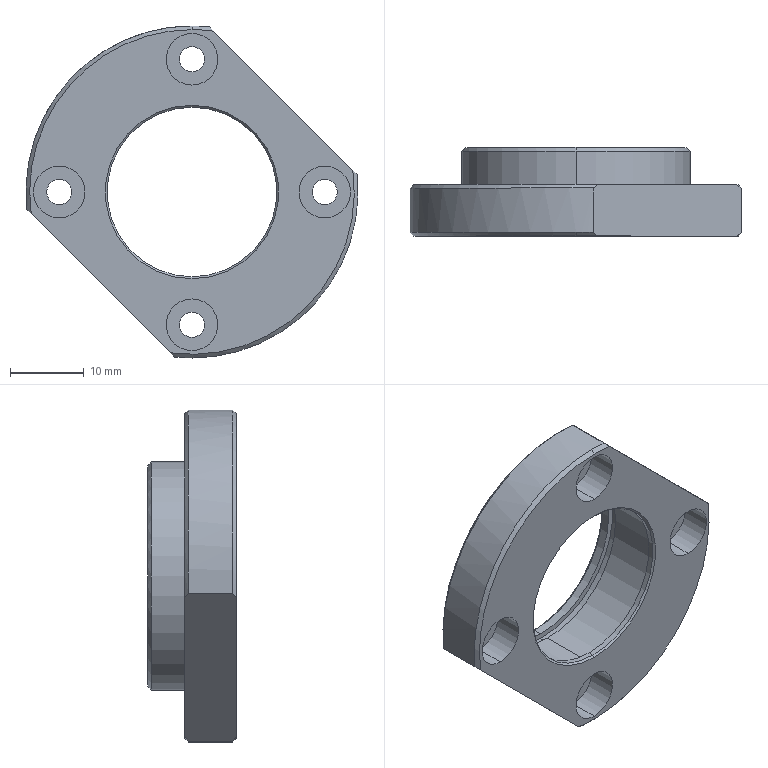Part | NX | features BREP 1 | 1 solid | 53 faces | box 45 x 12 x 45 mm | volume 6444 mm3 | cylinder 29 | plane 12 | cone 12 | commonest cylinder face diameters 3.4 x8 7 x8 26 x4 45 x3 23 x2 27.5 x2
STEP:
#1=CARTESIAN_POINT('',(21.802,0.,2.947));
#2=VERTEX_POINT('',#1);
#3=CARTESIAN_POINT('',(22.374,0.5,2.374));
#4=VERTEX_POINT('',#3);
#5=CARTESIAN_POINT('',(21.802,0.,2.947));
#6=CARTESIAN_POINT('',(21.994,0.1645,2.755));
#7=CARTESIAN_POINT('',(22.184,0.3312,2.564));
#8=CARTESIAN_POINT('',(22.374,0.5,2.374));
#9=B_SPLINE_CURVE_WITH_KNOTS('',3,(#5,#6,#7,#8),.UNSPECIFIED.,.F.,.F.,(4,4),(0.05986,0.06082),.UNSPECIFIED.);
#10=EDGE_CURVE('',#2,#4,#9,.T.);
#11=ORIENTED_EDGE('',*,*,#10,.T.);
#12=CARTESIAN_POINT('',(22.374,6.5,2.374));
#13=VERTEX_POINT('',#12);
#14=CARTESIAN_POINT('',(22.374,0.,2.374));
#15=DIRECTION('',(0.,-1.,0.));
#16=VECTOR('',#15,1000.);
#17=LINE('',#14,#16);
#18=EDGE_CURVE('',#13,#4,#17,.T.);
#19=ORIENTED_EDGE('',*,*,#18,.F.);
#20=CARTESIAN_POINT('',(21.802,7.,2.947));
#21=VERTEX_POINT('',#20);
#22=CARTESIAN_POINT('',(22.374,6.5,2.374));
#23=CARTESIAN_POINT('',(22.185,6.669,2.564));
#24=CARTESIAN_POINT('',(21.994,6.835,2.755));
#25=CARTESIAN_POINT('',(21.802,7.,2.947));
#26=B_SPLINE_CURVE_WITH_KNOTS('',3,(#22,#23,#24,#25),.UNSPECIFIED.,.F.,.F.,(4,4),(0.0304,0.03135),.UNSPECIFIED.);
#27=EDGE_CURVE('',#13,#21,#26,.T.);
#28=ORIENTED_EDGE('',*,*,#27,.T.);
#29=CARTESIAN_POINT('',(2.947,7.,21.802));
#30=VERTEX_POINT('',#29);
#31=CARTESIAN_POINT('',(4.624,7.,20.124));
#32=DIRECTION('',(0.7071,0.,-0.7071));
#33=VECTOR('',#32,1000.);
#34=LINE('',#31,#33);
#35=EDGE_CURVE('',#30,#21,#34,.T.);
#36=ORIENTED_EDGE('',*,*,#35,.F.);
#37=CARTESIAN_POINT('',(2.374,6.5,22.374));
#38=VERTEX_POINT('',#37);
#39=CARTESIAN_POINT('',(2.947,7.,21.802));
#40=CARTESIAN_POINT('',(2.755,6.836,21.994));
#41=CARTESIAN_POINT('',(2.564,6.669,22.184));
#42=CARTESIAN_POINT('',(2.374,6.5,22.374));
#43=B_SPLINE_CURVE_WITH_KNOTS('',3,(#39,#40,#41,#42),.UNSPECIFIED.,.F.,.F.,(4,4),(0.05986,0.06082),.UNSPECIFIED.);
#44=EDGE_CURVE('',#30,#38,#43,.T.);
#45=ORIENTED_EDGE('',*,*,#44,.T.);
#46=CARTESIAN_POINT('',(2.374,0.5,22.374));
#47=VERTEX_POINT('',#46);
#48=CARTESIAN_POINT('',(2.374,0.,22.374));
#49=DIRECTION('',(0.,1.,0.));
#50=VECTOR('',#49,1000.);
#51=LINE('',#48,#50);
#52=EDGE_CURVE('',#47,#38,#51,.T.);
#53=ORIENTED_EDGE('',*,*,#52,.F.);
#54=CARTESIAN_POINT('',(2.947,0.,21.802));
#55=VERTEX_POINT('',#54);
#56=CARTESIAN_POINT('',(2.374,0.5,22.374));
#57=CARTESIAN_POINT('',(2.564,0.3312,22.185));
#58=CARTESIAN_POINT('',(2.755,0.1645,21.994));
#59=CARTESIAN_POINT('',(2.947,0.,21.802));
#60=B_SPLINE_CURVE_WITH_KNOTS('',3,(#56,#57,#58,#59),.UNSPECIFIED.,.F.,.F.,(4,4),(0.0304,0.03135),.UNSPECIFIED.);
#61=EDGE_CURVE('',#47,#55,#60,.T.);
#62=ORIENTED_EDGE('',*,*,#61,.T.);
#63=CARTESIAN_POINT('',(0.,0.,24.749));
#64=DIRECTION('',(0.7071,0.,-0.7071));
#65=VECTOR('',#64,1000.);
#66=LINE('',#63,#65);
#67=EDGE_CURVE('',#55,#2,#66,.T.);
#68=ORIENTED_EDGE('',*,*,#67,.T.);
#69=EDGE_LOOP('',(#11,#19,#28,#36,#45,#53,#62,#68));
#70=FACE_BOUND('',#69,.T.);
#71=CARTESIAN_POINT('',(0.,23.,24.749));
#72=DIRECTION('',(-0.7071,0.,-0.7071));
#73=DIRECTION('',(-0.7071,0.,0.7071));
#74=AXIS2_PLACEMENT_3D('',#71,#72,#73);
#75=PLANE('',#74);
#76=ADVANCED_FACE('',(#70),#75,.F.);
#77=CARTESIAN_POINT('',(-21.802,0.,-2.947));
#78=VERTEX_POINT('',#77);
#79=CARTESIAN_POINT('',(-22.374,0.5,-2.374));
#80=VERTEX_POINT('',#79);
#81=CARTESIAN_POINT('',(-21.802,0.,-2.947));
#82=CARTESIAN_POINT('',(-21.994,0.1645,-2.755));
#83=CARTESIAN_POINT('',(-22.184,0.3312,-2.564));
#84=CARTESIAN_POINT('',(-22.374,0.5,-2.374));
#85=B_SPLINE_CURVE_WITH_KNOTS('',3,(#81,#82,#83,#84),.UNSPECIFIED.,.F.,.F.,(4,4),(0.05986,0.06082),.UNSPECIFIED.);
#86=EDGE_CURVE('',#78,#80,#85,.T.);
#87=ORIENTED_EDGE('',*,*,#86,.T.);
#88=CARTESIAN_POINT('',(-22.374,6.5,-2.374));
#89=VERTEX_POINT('',#88);
#90=CARTESIAN_POINT('',(-22.374,0.,-2.374));
#91=DIRECTION('',(0.,-1.,0.));
#92=VECTOR('',#91,1000.);
#93=LINE('',#90,#92);
#94=EDGE_CURVE('',#89,#80,#93,.T.);
#95=ORIENTED_EDGE('',*,*,#94,.F.);
#96=CARTESIAN_POINT('',(-21.802,7.,-2.947));
#97=VERTEX_POINT('',#96);
#98=CARTESIAN_POINT('',(-22.374,6.5,-2.374));
#99=CARTESIAN_POINT('',(-22.185,6.669,-2.564));
#100=CARTESIAN_POINT('',(-21.994,6.835,-2.755));
#101=CARTESIAN_POINT('',(-21.802,7.,-2.947));
#102=B_SPLINE_CURVE_WITH_KNOTS('',3,(#98,#99,#100,#101),.UNSPECIFIED.,.F.,.F.,(4,4),(0.0304,0.03135),.UNSPECIFIED.);
#103=EDGE_CURVE('',#89,#97,#102,.T.);
#104=ORIENTED_EDGE('',*,*,#103,.T.);
#105=CARTESIAN_POINT('',(-2.947,7.,-21.802));
#106=VERTEX_POINT('',#105);
#107=CARTESIAN_POINT('',(-20.124,7.,-4.624));
#108=DIRECTION('',(-0.7071,0.,0.7071));
#109=VECTOR('',#108,1000.);
#110=LINE('',#107,#109);
#111=EDGE_CURVE('',#106,#97,#110,.T.);
#112=ORIENTED_EDGE('',*,*,#111,.F.);
#113=CARTESIAN_POINT('',(-2.374,6.5,-22.374));
#114=VERTEX_POINT('',#113);
#115=CARTESIAN_POINT('',(-2.947,7.,-21.802));
#116=CARTESIAN_POINT('',(-2.755,6.836,-21.994));
#117=CARTESIAN_POINT('',(-2.564,6.669,-22.184));
#118=CARTESIAN_POINT('',(-2.374,6.5,-22.374));
#119=B_SPLINE_CURVE_WITH_KNOTS('',3,(#115,#116,#117,#118),.UNSPECIFIED.,.F.,.F.,(4,4),(0.05986,0.06082),.UNSPECIFIED.);
#120=EDGE_CURVE('',#106,#114,#119,.T.);
#121=ORIENTED_EDGE('',*,*,#120,.T.);
#122=CARTESIAN_POINT('',(-2.374,0.5,-22.374));
#123=VERTEX_POINT('',#122);
#124=CARTESIAN_POINT('',(-2.374,0.,-22.374));
#125=DIRECTION('',(0.,1.,0.));
#126=VECTOR('',#125,1000.);
#127=LINE('',#124,#126);
#128=EDGE_CURVE('',#123,#114,#127,.T.);
#129=ORIENTED_EDGE('',*,*,#128,.F.);
#130=CARTESIAN_POINT('',(-2.947,0.,-21.802));
#131=VERTEX_POINT('',#130);
#132=CARTESIAN_POINT('',(-2.374,0.5,-22.374));
#133=CARTESIAN_POINT('',(-2.564,0.3312,-22.185));
#134=CARTESIAN_POINT('',(-2.755,0.1645,-21.994));
#135=CARTESIAN_POINT('',(-2.947,0.,-21.802));
#136=B_SPLINE_CURVE_WITH_KNOTS('',3,(#132,#133,#134,#135),.UNSPECIFIED.,.F.,.F.,(4,4),(0.0304,0.03135),.UNSPECIFIED.);
#137=EDGE_CURVE('',#123,#131,#136,.T.);
#138=ORIENTED_EDGE('',*,*,#137,.T.);
#139=CARTESIAN_POINT('',(-24.749,0.,0.));
#140=DIRECTION('',(-0.7071,0.,0.7071));
#141=VECTOR('',#140,1000.);
#142=LINE('',#139,#141);
#143=EDGE_CURVE('',#131,#78,#142,.T.);
#144=ORIENTED_EDGE('',*,*,#143,.T.);
#145=EDGE_LOOP('',(#87,#95,#104,#112,#121,#129,#138,#144));
#146=FACE_BOUND('',#145,.T.);
#147=CARTESIAN_POINT('',(-24.749,23.,0.));
#148=DIRECTION('',(0.7071,0.,0.7071));
#149=DIRECTION('',(0.7071,0.,-0.7071));
#150=AXIS2_PLACEMENT_3D('',#147,#148,#149);
#151=PLANE('',#150);
#152=ADVANCED_FACE('',(#146),#151,.F.);
#153=CARTESIAN_POINT('',(0.,0.25,11.5));
#154=VERTEX_POINT('',#153);
#155=CARTESIAN_POINT('',(0.,0.,11.75));
#156=VERTEX_POINT('',#155);
#157=CARTESIAN_POINT('',(0.,0.25,11.5));
#158=DIRECTION('',(0.,-0.7071,0.7071));
#159=VECTOR('',#158,1000.);
#160=LINE('',#157,#159);
#161=EDGE_CURVE('',#154,#156,#160,.T.);
#162=ORIENTED_EDGE('',*,*,#161,.F.);
#163=CARTESIAN_POINT('',(0.,0.25,-11.5));
#164=VERTEX_POINT('',#163);
#165=CARTESIAN_POINT('',(0.,0.25,0.));
#166=DIRECTION('',(0.,-1.,0.));
#167=DIRECTION('',(0.,0.,1.));
#168=AXIS2_PLACEMENT_3D('',#165,#166,#167);
#169=CIRCLE('',#168,11.5);
#170=EDGE_CURVE('',#164,#154,#169,.T.);
#171=ORIENTED_EDGE('',*,*,#170,.F.);
#172=CARTESIAN_POINT('',(0.,0.,-11.75));
#173=VERTEX_POINT('',#172);
#174=CARTESIAN_POINT('',(0.,0.25,-11.5));
#175=DIRECTION('',(0.,-0.7071,-0.7071));
#176=VECTOR('',#175,1000.);
#177=LINE('',#174,#176);
#178=EDGE_CURVE('',#164,#173,#177,.T.);
#179=ORIENTED_EDGE('',*,*,#178,.T.);
#180=CARTESIAN_POINT('',(0.,0.,0.));
#181=DIRECTION('',(0.,1.,0.));
#182=DIRECTION('',(0.,0.,1.));
#183=AXIS2_PLACEMENT_3D('',#180,#181,#182);
#184=CIRCLE('',#183,11.75);
#185=EDGE_CURVE('',#156,#173,#184,.T.);
#186=ORIENTED_EDGE('',*,*,#185,.F.);
#187=EDGE_LOOP('',(#162,#171,#179,#186));
#188=FACE_BOUND('',#187,.T.);
#189=CARTESIAN_POINT('',(0.,0.25,0.));
#190=DIRECTION('',(0.,-1.,0.));
#191=DIRECTION('',(0.,0.,-1.));
#192=AXIS2_PLACEMENT_3D('',#189,#190,#191);
#193=CONICAL_SURFACE('',#192,11.5,0.7854);
#194=ADVANCED_FACE('',(#188),#193,.F.);
#195=CARTESIAN_POINT('',(0.,12.,15.));
#196=VERTEX_POINT('',#195);
#197=CARTESIAN_POINT('',(0.,11.5,15.5));
#198=VERTEX_POINT('',#197);
#199=CARTESIAN_POINT('',(0.,11.5,15.5));
#200=DIRECTION('',(0.,-0.7071,0.7071));
#201=VECTOR('',#200,1000.);
#202=LINE('',#199,#201);
#203=EDGE_CURVE('',#196,#198,#202,.T.);
#204=ORIENTED_EDGE('',*,*,#203,.F.);
#205=CARTESIAN_POINT('',(0.,12.,-15.));
#206=VERTEX_POINT('',#205);
#207=CARTESIAN_POINT('',(0.,12.,0.));
#208=DIRECTION('',(0.,1.,0.));
#209=DIRECTION('',(0.,0.,-1.));
#210=AXIS2_PLACEMENT_3D('',#207,#208,#209);
#211=CIRCLE('',#210,15.);
#212=EDGE_CURVE('',#206,#196,#211,.T.);
#213=ORIENTED_EDGE('',*,*,#212,.F.);
#214=CARTESIAN_POINT('',(0.,11.5,-15.5));
#215=VERTEX_POINT('',#214);
#216=CARTESIAN_POINT('',(0.,11.5,-15.5));
#217=DIRECTION('',(0.,-0.7071,-0.7071));
#218=VECTOR('',#217,1000.);
#219=LINE('',#216,#218);
#220=EDGE_CURVE('',#206,#215,#219,.T.);
#221=ORIENTED_EDGE('',*,*,#220,.T.);
#222=CARTESIAN_POINT('',(0.,11.5,0.));
#223=DIRECTION('',(0.,-1.,0.));
#224=DIRECTION('',(0.,0.,-1.));
#225=AXIS2_PLACEMENT_3D('',#222,#223,#224);
#226=CIRCLE('',#225,15.5);
#227=EDGE_CURVE('',#198,#215,#226,.T.);
#228=ORIENTED_EDGE('',*,*,#227,.F.);
#229=EDGE_LOOP('',(#204,#213,#221,#228));
#230=FACE_BOUND('',#229,.T.);
#231=CARTESIAN_POINT('',(0.,11.5,0.));
#232=DIRECTION('',(0.,-1.,0.));
#233=DIRECTION('',(0.,0.,-1.));
#234=AXIS2_PLACEMENT_3D('',#231,#232,#233);
#235=CONICAL_SURFACE('',#234,15.5,0.7854);
#236=ADVANCED_FACE('',(#230),#235,.T.);
#237=CARTESIAN_POINT('',(0.,12.,-13.5));
#238=VERTEX_POINT('',#237);
#239=CARTESIAN_POINT('',(0.,11.5,-13.));
#240=VERTEX_POINT('',#239);
#241=CARTESIAN_POINT('',(0.,12.,-13.5));
#242=DIRECTION('',(0.,0.7071,-0.7071));
#243=VECTOR('',#242,1000.);
#244=LINE('',#241,#243);
#245=EDGE_CURVE('',#238,#240,#244,.F.);
#246=ORIENTED_EDGE('',*,*,#245,.T.);
#247=CARTESIAN_POINT('',(0.,11.5,13.));
#248=VERTEX_POINT('',#247);
#249=CARTESIAN_POINT('',(0.,11.5,0.));
#250=DIRECTION('',(0.,1.,0.));
#251=DIRECTION('',(0.,0.,-1.));
#252=AXIS2_PLACEMENT_3D('',#249,#250,#251);
#253=CIRCLE('',#252,13.);
#254=EDGE_CURVE('',#248,#240,#253,.T.);
#255=ORIENTED_EDGE('',*,*,#254,.F.);
#256=CARTESIAN_POINT('',(0.,12.,13.5));
#257=VERTEX_POINT('',#256);
#258=CARTESIAN_POINT('',(0.,12.,13.5));
#259=DIRECTION('',(0.,0.7071,0.7071));
#260=VECTOR('',#259,1000.);
#261=LINE('',#258,#260);
#262=EDGE_CURVE('',#257,#248,#261,.F.);
#263=ORIENTED_EDGE('',*,*,#262,.F.);
#264=CARTESIAN_POINT('',(0.,12.,0.));
#265=DIRECTION('',(0.,-1.,0.));
#266=DIRECTION('',(0.,0.,-1.));
#267=AXIS2_PLACEMENT_3D('',#264,#265,#266);
#268=CIRCLE('',#267,13.5);
#269=EDGE_CURVE('',#238,#257,#268,.T.);
#270=ORIENTED_EDGE('',*,*,#269,.F.);
#271=EDGE_LOOP('',(#246,#255,#263,#270));
#272=FACE_BOUND('',#271,.T.);
#273=CARTESIAN_POINT('',(0.,12.,0.));
#274=DIRECTION('',(0.,1.,0.));
#275=DIRECTION('',(0.,0.,1.));
#276=AXIS2_PLACEMENT_3D('',#273,#274,#275);
#277=CONICAL_SURFACE('',#276,13.5,0.7854);
#278=ADVANCED_FACE('',(#272),#277,.F.);
#279=ORIENTED_EDGE('',*,*,#44,.F.);
#280=CARTESIAN_POINT('',(0.,7.,0.));
#281=DIRECTION('',(0.,1.,0.));
#282=DIRECTION('',(0.,0.,-1.));
#283=AXIS2_PLACEMENT_3D('',#280,#281,#282);
#284=CIRCLE('',#283,22.);
#285=EDGE_CURVE('',#97,#30,#284,.T.);
#286=ORIENTED_EDGE('',*,*,#285,.F.);
#287=ORIENTED_EDGE('',*,*,#103,.F.);
#288=CARTESIAN_POINT('',(0.,6.5,0.));
#289=DIRECTION('',(0.,-1.,0.));
#290=DIRECTION('',(0.,0.,-1.));
#291=AXIS2_PLACEMENT_3D('',#288,#289,#290);
#292=CIRCLE('',#291,22.5);
#293=EDGE_CURVE('',#38,#89,#292,.T.);
#294=ORIENTED_EDGE('',*,*,#293,.F.);
#295=EDGE_LOOP('',(#279,#286,#287,#294));
#296=FACE_BOUND('',#295,.T.);
#297=CARTESIAN_POINT('',(0.,6.5,0.));
#298=DIRECTION('',(0.,-1.,0.));
#299=DIRECTION('',(0.,0.,-1.));
#300=AXIS2_PLACEMENT_3D('',#297,#298,#299);
#301=CONICAL_SURFACE('',#300,22.5,0.7854);
#302=ADVANCED_FACE('',(#296),#301,.T.);
#303=ORIENTED_EDGE('',*,*,#10,.F.);
#304=CARTESIAN_POINT('',(0.,0.,0.));
#305=DIRECTION('',(0.,-1.,0.));
#306=DIRECTION('',(0.,0.,1.));
#307=AXIS2_PLACEMENT_3D('',#304,#305,#306);
#308=CIRCLE('',#307,22.);
#309=EDGE_CURVE('',#131,#2,#308,.T.);
#310=ORIENTED_EDGE('',*,*,#309,.F.);
#311=ORIENTED_EDGE('',*,*,#137,.F.);
#312=CARTESIAN_POINT('',(0.,0.5,-22.5));
#313=VERTEX_POINT('',#312);
#314=CARTESIAN_POINT('',(0.,0.5,0.));
#315=DIRECTION('',(0.,1.,0.));
#316=DIRECTION('',(0.,0.,1.));
#317=AXIS2_PLACEMENT_3D('',#314,#315,#316);
#318=CIRCLE('',#317,22.5);
#319=EDGE_CURVE('',#313,#123,#318,.T.);
#320=ORIENTED_EDGE('',*,*,#319,.F.);
#321=CARTESIAN_POINT('',(0.,0.5,0.));
#322=DIRECTION('',(0.,1.,0.));
#323=DIRECTION('',(0.,0.,1.));
#324=AXIS2_PLACEMENT_3D('',#321,#322,#323);
#325=CIRCLE('',#324,22.5);
#326=EDGE_CURVE('',#4,#313,#325,.T.);
#327=ORIENTED_EDGE('',*,*,#326,.F.);
#328=EDGE_LOOP('',(#303,#310,#311,#320,#327));
#329=FACE_BOUND('',#328,.T.);
#330=CARTESIAN_POINT('',(0.,0.,0.));
#331=DIRECTION('',(0.,1.,0.));
#332=DIRECTION('',(0.,0.,1.));
#333=AXIS2_PLACEMENT_3D('',#330,#331,#332);
#334=CONICAL_SURFACE('',#333,22.,0.7854);
#335=ADVANCED_FACE('',(#329),#334,.T.);
#336=CARTESIAN_POINT('',(0.,4.,-14.5));
#337=VERTEX_POINT('',#336);
#338=CARTESIAN_POINT('',(0.,0.,-14.5));
#339=VERTEX_POINT('',#338);
#340=CARTESIAN_POINT('',(0.,0.,-14.5));
#341=DIRECTION('',(0.,-1.,0.));
#342=VECTOR('',#341,1000.);
#343=LINE('',#340,#342);
#344=EDGE_CURVE('',#337,#339,#343,.T.);
#345=ORIENTED_EDGE('',*,*,#344,.F.);
#346=CARTESIAN_POINT('',(0.,4.,-21.5));
#347=VERTEX_POINT('',#346);
#348=CARTESIAN_POINT('',(0.,4.,-18.));
#349=DIRECTION('',(0.,-1.,0.));
#350=DIRECTION('',(0.,0.,-1.));
#351=AXIS2_PLACEMENT_3D('',#348,#349,#350);
#352=CIRCLE('',#351,3.5);
#353=EDGE_CURVE('',#347,#337,#352,.T.);
#354=ORIENTED_EDGE('',*,*,#353,.F.);
#355=CARTESIAN_POINT('',(0.,0.,-21.5));
#356=VERTEX_POINT('',#355);
#357=CARTESIAN_POINT('',(0.,0.,-21.5));
#358=DIRECTION('',(0.,-1.,0.));
#359=VECTOR('',#358,1000.);
#360=LINE('',#357,#359);
#361=EDGE_CURVE('',#347,#356,#360,.T.);
#362=ORIENTED_EDGE('',*,*,#361,.T.);
#363=CARTESIAN_POINT('',(0.,0.,-18.));
#364=DIRECTION('',(0.,-1.,0.));
#365=DIRECTION('',(0.,0.,-1.));
#366=AXIS2_PLACEMENT_3D('',#363,#364,#365);
#367=CIRCLE('',#366,3.5);
#368=EDGE_CURVE('',#356,#339,#367,.T.);
#369=ORIENTED_EDGE('',*,*,#368,.T.);
#370=EDGE_LOOP('',(#345,#354,#362,#369));
#371=FACE_BOUND('',#370,.T.);
#372=CARTESIAN_POINT('',(0.,0.,-18.));
#373=DIRECTION('',(0.,-1.,0.));
#374=DIRECTION('',(0.,0.,-1.));
#375=AXIS2_PLACEMENT_3D('',#372,#373,#374);
#376=CYLINDRICAL_SURFACE('',#375,3.5);
#377=ADVANCED_FACE('',(#371),#376,.F.);
#378=ORIENTED_EDGE('',*,*,#353,.T.);
#379=CARTESIAN_POINT('',(0.,4.,-18.));
#380=DIRECTION('',(0.,-1.,0.));
#381=DIRECTION('',(0.,0.,-1.));
#382=AXIS2_PLACEMENT_3D('',#379,#380,#381);
#383=CIRCLE('',#382,3.5);
#384=EDGE_CURVE('',#337,#347,#383,.T.);
#385=ORIENTED_EDGE('',*,*,#384,.T.);
#386=EDGE_LOOP('',(#378,#385));
#387=FACE_BOUND('',#386,.T.);
#388=CARTESIAN_POINT('',(0.,4.,-19.7));
#389=VERTEX_POINT('',#388);
#390=CARTESIAN_POINT('',(0.,4.,-16.3));
#391=VERTEX_POINT('',#390);
#392=CARTESIAN_POINT('',(0.,4.,-18.));
#393=DIRECTION('',(0.,-1.,0.));
#394=DIRECTION('',(0.,0.,-1.));
#395=AXIS2_PLACEMENT_3D('',#392,#393,#394);
#396=CIRCLE('',#395,1.7);
#397=EDGE_CURVE('',#389,#391,#396,.T.);
#398=ORIENTED_EDGE('',*,*,#397,.F.);
#399=CARTESIAN_POINT('',(0.,4.,-18.));
#400=DIRECTION('',(0.,-1.,0.));
#401=DIRECTION('',(0.,0.,-1.));
#402=AXIS2_PLACEMENT_3D('',#399,#400,#401);
#403=CIRCLE('',#402,1.7);
#404=EDGE_CURVE('',#391,#389,#403,.T.);
#405=ORIENTED_EDGE('',*,*,#404,.F.);
#406=EDGE_LOOP('',(#398,#405));
#407=FACE_BOUND('',#406,.T.);
#408=CARTESIAN_POINT('',(1.7,4.,-18.));
#409=DIRECTION('',(0.,1.,0.));
#410=DIRECTION('',(0.,0.,1.));
#411=AXIS2_PLACEMENT_3D('',#408,#409,#410);
#412=PLANE('',#411);
#413=ADVANCED_FACE('',(#387,#407),#412,.F.);
#414=CARTESIAN_POINT('',(0.,7.,-16.3));
#415=VERTEX_POINT('',#414);
#416=CARTESIAN_POINT('',(0.,0.,-16.3));
#417=DIRECTION('',(0.,-1.,0.));
#418=VECTOR('',#417,1000.);
#419=LINE('',#416,#418);
#420=EDGE_CURVE('',#415,#391,#419,.T.);
#421=ORIENTED_EDGE('',*,*,#420,.F.);
#422=CARTESIAN_POINT('',(0.,7.,-19.7));
#423=VERTEX_POINT('',#422);
#424=CARTESIAN_POINT('',(0.,7.,-18.));
#425=DIRECTION('',(0.,-1.,0.));
#426=DIRECTION('',(0.,0.,-1.));
#427=AXIS2_PLACEMENT_3D('',#424,#425,#426);
#428=CIRCLE('',#427,1.7);
#429=EDGE_CURVE('',#423,#415,#428,.T.);
#430=ORIENTED_EDGE('',*,*,#429,.F.);
#431=CARTESIAN_POINT('',(0.,0.,-19.7));
#432=DIRECTION('',(0.,-1.,0.));
#433=VECTOR('',#432,1000.);
#434=LINE('',#431,#433);
#435=EDGE_CURVE('',#423,#389,#434,.T.);
#436=ORIENTED_EDGE('',*,*,#435,.T.);
#437=ORIENTED_EDGE('',*,*,#397,.T.);
#438=EDGE_LOOP('',(#421,#430,#436,#437));
#439=FACE_BOUND('',#438,.T.);
#440=CARTESIAN_POINT('',(0.,0.,-18.));
#441=DIRECTION('',(0.,-1.,0.));
#442=DIRECTION('',(0.,0.,-1.));
#443=AXIS2_PLACEMENT_3D('',#440,#441,#442);
#444=CYLINDRICAL_SURFACE('',#443,1.7);
#445=ADVANCED_FACE('',(#439),#444,.F.);
#446=CARTESIAN_POINT('',(-18.,4.,3.5));
#447=VERTEX_POINT('',#446);
#448=CARTESIAN_POINT('',(-18.,0.,3.5));
#449=VERTEX_POINT('',#448);
#450=CARTESIAN_POINT('',(-18.,0.,3.5));
#451=DIRECTION('',(0.,-1.,0.));
#452=VECTOR('',#451,1000.);
#453=LINE('',#450,#452);
#454=EDGE_CURVE('',#447,#449,#453,.T.);
#455=ORIENTED_EDGE('',*,*,#454,.F.);
#456=CARTESIAN_POINT('',(-18.,4.,-3.5));
#457=VERTEX_POINT('',#456);
#458=CARTESIAN_POINT('',(-18.,4.,0.));
#459=DIRECTION('',(0.,-1.,0.));
#460=DIRECTION('',(0.,0.,-1.));
#461=AXIS2_PLACEMENT_3D('',#458,#459,#460);
#462=CIRCLE('',#461,3.5);
#463=EDGE_CURVE('',#457,#447,#462,.T.);
#464=ORIENTED_EDGE('',*,*,#463,.F.);
#465=CARTESIAN_POINT('',(-18.,0.,-3.5));
#466=VERTEX_POINT('',#465);
#467=CARTESIAN_POINT('',(-18.,0.,-3.5));
#468=DIRECTION('',(0.,-1.,0.));
#469=VECTOR('',#468,1000.);
#470=LINE('',#467,#469);
#471=EDGE_CURVE('',#457,#466,#470,.T.);
#472=ORIENTED_EDGE('',*,*,#471,.T.);
#473=CARTESIAN_POINT('',(-18.,0.,0.));
#474=DIRECTION('',(0.,-1.,0.));
#475=DIRECTION('',(0.,0.,-1.));
#476=AXIS2_PLACEMENT_3D('',#473,#474,#475);
#477=CIRCLE('',#476,3.5);
#478=EDGE_CURVE('',#466,#449,#477,.T.);
#479=ORIENTED_EDGE('',*,*,#478,.T.);
#480=EDGE_LOOP('',(#455,#464,#472,#479));
#481=FACE_BOUND('',#480,.T.);
#482=CARTESIAN_POINT('',(-18.,0.,0.));
#483=DIRECTION('',(0.,-1.,0.));
#484=DIRECTION('',(0.,0.,-1.));
#485=AXIS2_PLACEMENT_3D('',#482,#483,#484);
#486=CYLINDRICAL_SURFACE('',#485,3.5);
#487=ADVANCED_FACE('',(#481),#486,.F.);
#488=ORIENTED_EDGE('',*,*,#463,.T.);
#489=CARTESIAN_POINT('',(-18.,4.,0.));
#490=DIRECTION('',(0.,-1.,0.));
#491=DIRECTION('',(0.,0.,-1.));
#492=AXIS2_PLACEMENT_3D('',#489,#490,#491);
#493=CIRCLE('',#492,3.5);
#494=EDGE_CURVE('',#447,#457,#493,.T.);
#495=ORIENTED_EDGE('',*,*,#494,.T.);
#496=EDGE_LOOP('',(#488,#495));
#497=FACE_BOUND('',#496,.T.);
#498=CARTESIAN_POINT('',(-18.,4.,-1.7));
#499=VERTEX_POINT('',#498);
#500=CARTESIAN_POINT('',(-18.,4.,1.7));
#501=VERTEX_POINT('',#500);
#502=CARTESIAN_POINT('',(-18.,4.,0.));
#503=DIRECTION('',(0.,-1.,0.));
#504=DIRECTION('',(0.,0.,-1.));
#505=AXIS2_PLACEMENT_3D('',#502,#503,#504);
#506=CIRCLE('',#505,1.7);
#507=EDGE_CURVE('',#499,#501,#506,.T.);
#508=ORIENTED_EDGE('',*,*,#507,.F.);
#509=CARTESIAN_POINT('',(-18.,4.,0.));
#510=DIRECTION('',(0.,-1.,0.));
#511=DIRECTION('',(0.,0.,-1.));
#512=AXIS2_PLACEMENT_3D('',#509,#510,#511);
#513=CIRCLE('',#512,1.7);
#514=EDGE_CURVE('',#501,#499,#513,.T.);
#515=ORIENTED_EDGE('',*,*,#514,.F.);
#516=EDGE_LOOP('',(#508,#515));
#517=FACE_BOUND('',#516,.T.);
#518=CARTESIAN_POINT('',(-16.3,4.,0.));
#519=DIRECTION('',(0.,1.,0.));
#520=DIRECTION('',(0.,0.,1.));
#521=AXIS2_PLACEMENT_3D('',#518,#519,#520);
#522=PLANE('',#521);
#523=ADVANCED_FACE('',(#497,#517),#522,.F.);
#524=CARTESIAN_POINT('',(-18.,7.,1.7));
#525=VERTEX_POINT('',#524);
#526=CARTESIAN_POINT('',(-18.,0.,1.7));
#527=DIRECTION('',(0.,-1.,0.));
#528=VECTOR('',#527,1000.);
#529=LINE('',#526,#528);
#530=EDGE_CURVE('',#525,#501,#529,.T.);
#531=ORIENTED_EDGE('',*,*,#530,.F.);
#532=CARTESIAN_POINT('',(-18.,7.,-1.7));
#533=VERTEX_POINT('',#532);
#534=CARTESIAN_POINT('',(-18.,7.,0.));
#535=DIRECTION('',(0.,-1.,0.));
#536=DIRECTION('',(0.,0.,-1.));
#537=AXIS2_PLACEMENT_3D('',#534,#535,#536);
#538=CIRCLE('',#537,1.7);
#539=EDGE_CURVE('',#533,#525,#538,.T.);
#540=ORIENTED_EDGE('',*,*,#539,.F.);
#541=CARTESIAN_POINT('',(-18.,0.,-1.7));
#542=DIRECTION('',(0.,-1.,0.));
#543=VECTOR('',#542,1000.);
#544=LINE('',#541,#543);
#545=EDGE_CURVE('',#533,#499,#544,.T.);
#546=ORIENTED_EDGE('',*,*,#545,.T.);
#547=ORIENTED_EDGE('',*,*,#507,.T.);
#548=EDGE_LOOP('',(#531,#540,#546,#547));
#549=FACE_BOUND('',#548,.T.);
#550=CARTESIAN_POINT('',(-18.,0.,0.));
#551=DIRECTION('',(0.,-1.,0.));
#552=DIRECTION('',(0.,0.,-1.));
#553=AXIS2_PLACEMENT_3D('',#550,#551,#552);
#554=CYLINDRICAL_SURFACE('',#553,1.7);
#555=ADVANCED_FACE('',(#549),#554,.F.);
#556=CARTESIAN_POINT('',(0.,4.,21.5));
#557=VERTEX_POINT('',#556);
#558=CARTESIAN_POINT('',(0.,0.,21.5));
#559=VERTEX_POINT('',#558);
#560=CARTESIAN_POINT('',(0.,0.,21.5));
#561=DIRECTION('',(0.,-1.,0.));
#562=VECTOR('',#561,1000.);
#563=LINE('',#560,#562);
#564=EDGE_CURVE('',#557,#559,#563,.T.);
#565=ORIENTED_EDGE('',*,*,#564,.F.);
#566=CARTESIAN_POINT('',(0.,4.,14.5));
#567=VERTEX_POINT('',#566);
#568=CARTESIAN_POINT('',(0.,4.,18.));
#569=DIRECTION('',(0.,-1.,0.));
#570=DIRECTION('',(0.,0.,-1.));
#571=AXIS2_PLACEMENT_3D('',#568,#569,#570);
#572=CIRCLE('',#571,3.5);
#573=EDGE_CURVE('',#567,#557,#572,.T.);
#574=ORIENTED_EDGE('',*,*,#573,.F.);
#575=CARTESIAN_POINT('',(0.,0.,14.5));
#576=VERTEX_POINT('',#575);
#577=CARTESIAN_POINT('',(0.,0.,14.5));
#578=DIRECTION('',(0.,-1.,0.));
#579=VECTOR('',#578,1000.);
#580=LINE('',#577,#579);
#581=EDGE_CURVE('',#567,#576,#580,.T.);
#582=ORIENTED_EDGE('',*,*,#581,.T.);
#583=CARTESIAN_POINT('',(0.,0.,18.));
#584=DIRECTION('',(0.,-1.,0.));
#585=DIRECTION('',(0.,0.,-1.));
#586=AXIS2_PLACEMENT_3D('',#583,#584,#585);
#587=CIRCLE('',#586,3.5);
#588=EDGE_CURVE('',#576,#559,#587,.T.);
#589=ORIENTED_EDGE('',*,*,#588,.T.);
#590=EDGE_LOOP('',(#565,#574,#582,#589));
#591=FACE_BOUND('',#590,.T.);
#592=CARTESIAN_POINT('',(0.,0.,18.));
#593=DIRECTION('',(0.,-1.,0.));
#594=DIRECTION('',(0.,0.,-1.));
#595=AXIS2_PLACEMENT_3D('',#592,#593,#594);
#596=CYLINDRICAL_SURFACE('',#595,3.5);
#597=ADVANCED_FACE('',(#591),#596,.F.);
#598=ORIENTED_EDGE('',*,*,#573,.T.);
#599=CARTESIAN_POINT('',(0.,4.,18.));
#600=DIRECTION('',(0.,-1.,0.));
#601=DIRECTION('',(0.,0.,-1.));
#602=AXIS2_PLACEMENT_3D('',#599,#600,#601);
#603=CIRCLE('',#602,3.5);
#604=EDGE_CURVE('',#557,#567,#603,.T.);
#605=ORIENTED_EDGE('',*,*,#604,.T.);
#606=EDGE_LOOP('',(#598,#605));
#607=FACE_BOUND('',#606,.T.);
#608=CARTESIAN_POINT('',(0.,4.,16.3));
#609=VERTEX_POINT('',#608);
#610=CARTESIAN_POINT('',(0.,4.,19.7));
#611=VERTEX_POINT('',#610);
#612=CARTESIAN_POINT('',(0.,4.,18.));
#613=DIRECTION('',(0.,-1.,0.));
#614=DIRECTION('',(0.,0.,-1.));
#615=AXIS2_PLACEMENT_3D('',#612,#613,#614);
#616=CIRCLE('',#615,1.7);
#617=EDGE_CURVE('',#609,#611,#616,.T.);
#618=ORIENTED_EDGE('',*,*,#617,.F.);
#619=CARTESIAN_POINT('',(0.,4.,18.));
#620=DIRECTION('',(0.,-1.,0.));
#621=DIRECTION('',(0.,0.,-1.));
#622=AXIS2_PLACEMENT_3D('',#619,#620,#621);
#623=CIRCLE('',#622,1.7);
#624=EDGE_CURVE('',#611,#609,#623,.T.);
#625=ORIENTED_EDGE('',*,*,#624,.F.);
#626=EDGE_LOOP('',(#618,#625));
#627=FACE_BOUND('',#626,.T.);
#628=CARTESIAN_POINT('',(1.7,4.,18.));
#629=DIRECTION('',(0.,1.,0.));
#630=DIRECTION('',(0.,0.,1.));
#631=AXIS2_PLACEMENT_3D('',#628,#629,#630);
#632=PLANE('',#631);
#633=ADVANCED_FACE('',(#607,#627),#632,.F.);
#634=CARTESIAN_POINT('',(0.,7.,19.7));
#635=VERTEX_POINT('',#634);
#636=CARTESIAN_POINT('',(0.,0.,19.7));
#637=DIRECTION('',(0.,-1.,0.));
#638=VECTOR('',#637,1000.);
#639=LINE('',#636,#638);
#640=EDGE_CURVE('',#635,#611,#639,.T.);
#641=ORIENTED_EDGE('',*,*,#640,.F.);
#642=CARTESIAN_POINT('',(0.,7.,16.3));
#643=VERTEX_POINT('',#642);
#644=CARTESIAN_POINT('',(0.,7.,18.));
#645=DIRECTION('',(0.,-1.,0.));
#646=DIRECTION('',(0.,0.,-1.));
#647=AXIS2_PLACEMENT_3D('',#644,#645,#646);
#648=CIRCLE('',#647,1.7);
#649=EDGE_CURVE('',#643,#635,#648,.T.);
#650=ORIENTED_EDGE('',*,*,#649,.F.);
#651=CARTESIAN_POINT('',(0.,0.,16.3));
#652=DIRECTION('',(0.,-1.,0.));
#653=VECTOR('',#652,1000.);
#654=LINE('',#651,#653);
#655=EDGE_CURVE('',#643,#609,#654,.T.);
#656=ORIENTED_EDGE('',*,*,#655,.T.);
#657=ORIENTED_EDGE('',*,*,#617,.T.);
#658=EDGE_LOOP('',(#641,#650,#656,#657));
#659=FACE_BOUND('',#658,.T.);
#660=CARTESIAN_POINT('',(0.,0.,18.));
#661=DIRECTION('',(0.,-1.,0.));
#662=DIRECTION('',(0.,0.,-1.));
#663=AXIS2_PLACEMENT_3D('',#660,#661,#662);
#664=CYLINDRICAL_SURFACE('',#663,1.7);
#665=ADVANCED_FACE('',(#659),#664,.F.);
#666=CARTESIAN_POINT('',(18.,4.,3.5));
#667=VERTEX_POINT('',#666);
#668=CARTESIAN_POINT('',(18.,0.,3.5));
#669=VERTEX_POINT('',#668);
#670=CARTESIAN_POINT('',(18.,0.,3.5));
#671=DIRECTION('',(0.,-1.,0.));
#672=VECTOR('',#671,1000.);
#673=LINE('',#670,#672);
#674=EDGE_CURVE('',#667,#669,#673,.T.);
#675=ORIENTED_EDGE('',*,*,#674,.F.);
#676=CARTESIAN_POINT('',(18.,4.,-3.5));
#677=VERTEX_POINT('',#676);
#678=CARTESIAN_POINT('',(18.,4.,0.));
#679=DIRECTION('',(0.,-1.,0.));
#680=DIRECTION('',(0.,0.,-1.));
#681=AXIS2_PLACEMENT_3D('',#678,#679,#680);
#682=CIRCLE('',#681,3.5);
#683=EDGE_CURVE('',#677,#667,#682,.T.);
#684=ORIENTED_EDGE('',*,*,#683,.F.);
#685=CARTESIAN_POINT('',(18.,0.,-3.5));
#686=VERTEX_POINT('',#685);
#687=CARTESIAN_POINT('',(18.,0.,-3.5));
#688=DIRECTION('',(0.,-1.,0.));
#689=VECTOR('',#688,1000.);
#690=LINE('',#687,#689);
#691=EDGE_CURVE('',#677,#686,#690,.T.);
#692=ORIENTED_EDGE('',*,*,#691,.T.);
#693=CARTESIAN_POINT('',(18.,0.,0.));
#694=DIRECTION('',(0.,-1.,0.));
#695=DIRECTION('',(0.,0.,-1.));
#696=AXIS2_PLACEMENT_3D('',#693,#694,#695);
#697=CIRCLE('',#696,3.5);
#698=EDGE_CURVE('',#686,#669,#697,.T.);
#699=ORIENTED_EDGE('',*,*,#698,.T.);
#700=EDGE_LOOP('',(#675,#684,#692,#699));
#701=FACE_BOUND('',#700,.T.);
#702=CARTESIAN_POINT('',(18.,0.,0.));
#703=DIRECTION('',(0.,-1.,0.));
#704=DIRECTION('',(0.,0.,-1.));
#705=AXIS2_PLACEMENT_3D('',#702,#703,#704);
#706=CYLINDRICAL_SURFACE('',#705,3.5);
#707=ADVANCED_FACE('',(#701),#706,.F.);
#708=ORIENTED_EDGE('',*,*,#683,.T.);
#709=CARTESIAN_POINT('',(18.,4.,0.));
#710=DIRECTION('',(0.,-1.,0.));
#711=DIRECTION('',(0.,0.,-1.));
#712=AXIS2_PLACEMENT_3D('',#709,#710,#711);
#713=CIRCLE('',#712,3.5);
#714=EDGE_CURVE('',#667,#677,#713,.T.);
#715=ORIENTED_EDGE('',*,*,#714,.T.);
#716=EDGE_LOOP('',(#708,#715));
#717=FACE_BOUND('',#716,.T.);
#718=CARTESIAN_POINT('',(18.,4.,-1.7));
#719=VERTEX_POINT('',#718);
#720=CARTESIAN_POINT('',(18.,4.,1.7));
#721=VERTEX_POINT('',#720);
#722=CARTESIAN_POINT('',(18.,4.,0.));
#723=DIRECTION('',(0.,-1.,0.));
#724=DIRECTION('',(0.,0.,-1.));
#725=AXIS2_PLACEMENT_3D('',#722,#723,#724);
#726=CIRCLE('',#725,1.7);
#727=EDGE_CURVE('',#719,#721,#726,.T.);
#728=ORIENTED_EDGE('',*,*,#727,.F.);
#729=CARTESIAN_POINT('',(18.,4.,0.));
#730=DIRECTION('',(0.,-1.,0.));
#731=DIRECTION('',(0.,0.,-1.));
#732=AXIS2_PLACEMENT_3D('',#729,#730,#731);
#733=CIRCLE('',#732,1.7);
#734=EDGE_CURVE('',#721,#719,#733,.T.);
#735=ORIENTED_EDGE('',*,*,#734,.F.);
#736=EDGE_LOOP('',(#728,#735));
#737=FACE_BOUND('',#736,.T.);
#738=CARTESIAN_POINT('',(19.7,4.,0.));
#739=DIRECTION('',(0.,1.,0.));
#740=DIRECTION('',(0.,0.,1.));
#741=AXIS2_PLACEMENT_3D('',#738,#739,#740);
#742=PLANE('',#741);
#743=ADVANCED_FACE('',(#717,#737),#742,.F.);
#744=CARTESIAN_POINT('',(18.,7.,1.7));
#745=VERTEX_POINT('',#744);
#746=CARTESIAN_POINT('',(18.,0.,1.7));
#747=DIRECTION('',(0.,-1.,0.));
#748=VECTOR('',#747,1000.);
#749=LINE('',#746,#748);
#750=EDGE_CURVE('',#745,#721,#749,.T.);
#751=ORIENTED_EDGE('',*,*,#750,.F.);
#752=CARTESIAN_POINT('',(18.,7.,-1.7));
#753=VERTEX_POINT('',#752);
#754=CARTESIAN_POINT('',(18.,7.,0.));
#755=DIRECTION('',(0.,-1.,0.));
#756=DIRECTION('',(0.,0.,-1.));
#757=AXIS2_PLACEMENT_3D('',#754,#755,#756);
#758=CIRCLE('',#757,1.7);
#759=EDGE_CURVE('',#753,#745,#758,.T.);
#760=ORIENTED_EDGE('',*,*,#759,.F.);
#761=CARTESIAN_POINT('',(18.,0.,-1.7));
#762=DIRECTION('',(0.,-1.,0.));
#763=VECTOR('',#762,1000.);
#764=LINE('',#761,#763);
#765=EDGE_CURVE('',#753,#719,#764,.T.);
#766=ORIENTED_EDGE('',*,*,#765,.T.);
#767=ORIENTED_EDGE('',*,*,#727,.T.);
#768=EDGE_LOOP('',(#751,#760,#766,#767));
#769=FACE_BOUND('',#768,.T.);
#770=CARTESIAN_POINT('',(18.,0.,0.));
#771=DIRECTION('',(0.,-1.,0.));
#772=DIRECTION('',(0.,0.,-1.));
#773=AXIS2_PLACEMENT_3D('',#770,#771,#772);
#774=CYLINDRICAL_SURFACE('',#773,1.7);
#775=ADVANCED_FACE('',(#769),#774,.F.);
#776=CARTESIAN_POINT('',(0.,10.25,-13.75));
#777=VERTEX_POINT('',#776);
#778=CARTESIAN_POINT('',(0.,10.25,13.75));
#779=VERTEX_POINT('',#778);
#780=CARTESIAN_POINT('',(0.,10.25,0.));
#781=DIRECTION('',(0.,-1.,0.));
#782=DIRECTION('',(0.,0.,-1.));
#783=AXIS2_PLACEMENT_3D('',#780,#781,#782);
#784=CIRCLE('',#783,13.75);
#785=EDGE_CURVE('',#777,#779,#784,.T.);
#786=ORIENTED_EDGE('',*,*,#785,.T.);
#787=CARTESIAN_POINT('',(0.,10.25,0.));
#788=DIRECTION('',(0.,-1.,0.));
#789=DIRECTION('',(0.,0.,-1.));
#790=AXIS2_PLACEMENT_3D('',#787,#788,#789);
#791=CIRCLE('',#790,13.75);
#792=EDGE_CURVE('',#779,#777,#791,.T.);
#793=ORIENTED_EDGE('',*,*,#792,.T.);
#794=EDGE_LOOP('',(#786,#793));
#795=FACE_BOUND('',#794,.T.);
#796=CARTESIAN_POINT('',(0.,10.25,-13.));
#797=VERTEX_POINT('',#796);
#798=CARTESIAN_POINT('',(0.,10.25,13.));
#799=VERTEX_POINT('',#798);
#800=CARTESIAN_POINT('',(0.,10.25,0.));
#801=DIRECTION('',(0.,-1.,0.));
#802=DIRECTION('',(0.,0.,-1.));
#803=AXIS2_PLACEMENT_3D('',#800,#801,#802);
#804=CIRCLE('',#803,13.);
#805=EDGE_CURVE('',#797,#799,#804,.T.);
#806=ORIENTED_EDGE('',*,*,#805,.F.);
#807=CARTESIAN_POINT('',(0.,10.25,0.));
#808=DIRECTION('',(0.,-1.,0.));
#809=DIRECTION('',(0.,0.,-1.));
#810=AXIS2_PLACEMENT_3D('',#807,#808,#809);
#811=CIRCLE('',#810,13.);
#812=EDGE_CURVE('',#799,#797,#811,.T.);
#813=ORIENTED_EDGE('',*,*,#812,.F.);
#814=EDGE_LOOP('',(#806,#813));
#815=FACE_BOUND('',#814,.T.);
#816=CARTESIAN_POINT('',(-13.,10.25,0.));
#817=DIRECTION('',(0.,1.,0.));
#818=DIRECTION('',(0.,0.,1.));
#819=AXIS2_PLACEMENT_3D('',#816,#817,#818);
#820=PLANE('',#819);
#821=ADVANCED_FACE('',(#795,#815),#820,.F.);
#822=CARTESIAN_POINT('',(0.,8.9,13.75));
#823=VERTEX_POINT('',#822);
#824=CARTESIAN_POINT('',(0.,0.,13.75));
#825=DIRECTION('',(0.,-1.,0.));
#826=VECTOR('',#825,1000.);
#827=LINE('',#824,#826);
#828=EDGE_CURVE('',#779,#823,#827,.T.);
#829=ORIENTED_EDGE('',*,*,#828,.F.);
#830=ORIENTED_EDGE('',*,*,#785,.F.);
#831=CARTESIAN_POINT('',(0.,8.9,-13.75));
#832=VERTEX_POINT('',#831);
#833=CARTESIAN_POINT('',(0.,0.,-13.75));
#834=DIRECTION('',(0.,-1.,0.));
#835=VECTOR('',#834,1000.);
#836=LINE('',#833,#835);
#837=EDGE_CURVE('',#777,#832,#836,.T.);
#838=ORIENTED_EDGE('',*,*,#837,.T.);
#839=CARTESIAN_POINT('',(0.,8.9,0.));
#840=DIRECTION('',(0.,-1.,0.));
#841=DIRECTION('',(0.,0.,-1.));
#842=AXIS2_PLACEMENT_3D('',#839,#840,#841);
#843=CIRCLE('',#842,13.75);
#844=EDGE_CURVE('',#832,#823,#843,.T.);
#845=ORIENTED_EDGE('',*,*,#844,.T.);
#846=EDGE_LOOP('',(#829,#830,#838,#845));
#847=FACE_BOUND('',#846,.T.);
#848=CARTESIAN_POINT('',(0.,0.,0.));
#849=DIRECTION('',(0.,-1.,0.));
#850=DIRECTION('',(0.,0.,-1.));
#851=AXIS2_PLACEMENT_3D('',#848,#849,#850);
#852=CYLINDRICAL_SURFACE('',#851,13.75);
#853=ADVANCED_FACE('',(#847),#852,.F.);
#854=CARTESIAN_POINT('',(0.,8.9,-13.));
#855=VERTEX_POINT('',#854);
#856=CARTESIAN_POINT('',(0.,8.9,13.));
#857=VERTEX_POINT('',#856);
#858=CARTESIAN_POINT('',(0.,8.9,0.));
#859=DIRECTION('',(0.,-1.,0.));
#860=DIRECTION('',(0.,0.,-1.));
#861=AXIS2_PLACEMENT_3D('',#858,#859,#860);
#862=CIRCLE('',#861,13.);
#863=EDGE_CURVE('',#855,#857,#862,.T.);
#864=ORIENTED_EDGE('',*,*,#863,.T.);
#865=CARTESIAN_POINT('',(0.,8.9,0.));
#866=DIRECTION('',(0.,-1.,0.));
#867=DIRECTION('',(0.,0.,-1.));
#868=AXIS2_PLACEMENT_3D('',#865,#866,#867);
#869=CIRCLE('',#868,13.);
#870=EDGE_CURVE('',#857,#855,#869,.T.);
#871=ORIENTED_EDGE('',*,*,#870,.T.);
#872=EDGE_LOOP('',(#864,#871));
#873=FACE_BOUND('',#872,.T.);
#874=ORIENTED_EDGE('',*,*,#844,.F.);
#875=CARTESIAN_POINT('',(0.,8.9,0.));
#876=DIRECTION('',(0.,-1.,0.));
#877=DIRECTION('',(0.,0.,-1.));
#878=AXIS2_PLACEMENT_3D('',#875,#876,#877);
#879=CIRCLE('',#878,13.75);
#880=EDGE_CURVE('',#823,#832,#879,.T.);
#881=ORIENTED_EDGE('',*,*,#880,.F.);
#882=EDGE_LOOP('',(#874,#881));
#883=FACE_BOUND('',#882,.T.);
#884=CARTESIAN_POINT('',(-13.75,8.9,0.));
#885=DIRECTION('',(0.,-1.,0.));
#886=DIRECTION('',(0.,0.,-1.));
#887=AXIS2_PLACEMENT_3D('',#884,#885,#886);
#888=PLANE('',#887);
#889=ADVANCED_FACE('',(#873,#883),#888,.F.);
#890=CARTESIAN_POINT('',(0.,1.,13.));
#891=VERTEX_POINT('',#890);
#892=CARTESIAN_POINT('',(0.,0.,13.));
#893=DIRECTION('',(0.,-1.,0.));
#894=VECTOR('',#893,1000.);
#895=LINE('',#892,#894);
#896=EDGE_CURVE('',#857,#891,#895,.T.);
#897=ORIENTED_EDGE('',*,*,#896,.F.);
#898=ORIENTED_EDGE('',*,*,#863,.F.);
#899=CARTESIAN_POINT('',(0.,1.,-13.));
#900=VERTEX_POINT('',#899);
#901=CARTESIAN_POINT('',(0.,0.,-13.));
#902=DIRECTION('',(0.,-1.,0.));
#903=VECTOR('',#902,1000.);
#904=LINE('',#901,#903);
#905=EDGE_CURVE('',#855,#900,#904,.T.);
#906=ORIENTED_EDGE('',*,*,#905,.T.);
#907=CARTESIAN_POINT('',(0.,1.,0.));
#908=DIRECTION('',(0.,-1.,0.));
#909=DIRECTION('',(0.,0.,-1.));
#910=AXIS2_PLACEMENT_3D('',#907,#908,#909);
#911=CIRCLE('',#910,13.);
#912=EDGE_CURVE('',#900,#891,#911,.T.);
#913=ORIENTED_EDGE('',*,*,#912,.T.);
#914=EDGE_LOOP('',(#897,#898,#906,#913));
#915=FACE_BOUND('',#914,.T.);
#916=CARTESIAN_POINT('',(0.,0.,0.));
#917=DIRECTION('',(0.,-1.,0.));
#918=DIRECTION('',(0.,0.,-1.));
#919=AXIS2_PLACEMENT_3D('',#916,#917,#918);
#920=CYLINDRICAL_SURFACE('',#919,13.);
#921=ADVANCED_FACE('',(#915),#920,.F.);
#922=CARTESIAN_POINT('',(0.,1.,-11.5));
#923=VERTEX_POINT('',#922);
#924=CARTESIAN_POINT('',(0.,1.,11.5));
#925=VERTEX_POINT('',#924);
#926=CARTESIAN_POINT('',(0.,1.,0.));
#927=DIRECTION('',(0.,-1.,0.));
#928=DIRECTION('',(0.,0.,-1.));
#929=AXIS2_PLACEMENT_3D('',#926,#927,#928);
#930=CIRCLE('',#929,11.5);
#931=EDGE_CURVE('',#923,#925,#930,.T.);
#932=ORIENTED_EDGE('',*,*,#931,.T.);
#933=CARTESIAN_POINT('',(0.,1.,0.));
#934=DIRECTION('',(0.,-1.,0.));
#935=DIRECTION('',(0.,0.,-1.));
#936=AXIS2_PLACEMENT_3D('',#933,#934,#935);
#937=CIRCLE('',#936,11.5);
#938=EDGE_CURVE('',#925,#923,#937,.T.);
#939=ORIENTED_EDGE('',*,*,#938,.T.);
#940=EDGE_LOOP('',(#932,#939));
#941=FACE_BOUND('',#940,.T.);
#942=ORIENTED_EDGE('',*,*,#912,.F.);
#943=CARTESIAN_POINT('',(0.,1.,0.));
#944=DIRECTION('',(0.,-1.,0.));
#945=DIRECTION('',(0.,0.,-1.));
#946=AXIS2_PLACEMENT_3D('',#943,#944,#945);
#947=CIRCLE('',#946,13.);
#948=EDGE_CURVE('',#891,#900,#947,.T.);
#949=ORIENTED_EDGE('',*,*,#948,.F.);
#950=EDGE_LOOP('',(#942,#949));
#951=FACE_BOUND('',#950,.T.);
#952=CARTESIAN_POINT('',(-11.5,1.,0.));
#953=DIRECTION('',(0.,-1.,0.));
#954=DIRECTION('',(0.,0.,-1.));
#955=AXIS2_PLACEMENT_3D('',#952,#953,#954);
#956=PLANE('',#955);
#957=ADVANCED_FACE('',(#941,#951),#956,.F.);
#958=CARTESIAN_POINT('',(0.,0.,11.5));
#959=DIRECTION('',(0.,-1.,0.));
#960=VECTOR('',#959,1000.);
#961=LINE('',#958,#960);
#962=EDGE_CURVE('',#925,#154,#961,.T.);
#963=ORIENTED_EDGE('',*,*,#962,.F.);
#964=ORIENTED_EDGE('',*,*,#931,.F.);
#965=CARTESIAN_POINT('',(0.,0.,-11.5));
#966=DIRECTION('',(0.,-1.,0.));
#967=VECTOR('',#966,1000.);
#968=LINE('',#965,#967);
#969=EDGE_CURVE('',#923,#164,#968,.T.);
#970=ORIENTED_EDGE('',*,*,#969,.T.);
#971=ORIENTED_EDGE('',*,*,#170,.T.);
#972=EDGE_LOOP('',(#963,#964,#970,#971));
#973=FACE_BOUND('',#972,.T.);
#974=CARTESIAN_POINT('',(0.,0.,0.));
#975=DIRECTION('',(0.,-1.,0.));
#976=DIRECTION('',(0.,0.,-1.));
#977=AXIS2_PLACEMENT_3D('',#974,#975,#976);
#978=CYLINDRICAL_SURFACE('',#977,11.5);
#979=ADVANCED_FACE('',(#973),#978,.F.);
#980=ORIENTED_EDGE('',*,*,#698,.F.);
#981=CARTESIAN_POINT('',(18.,0.,0.));
#982=DIRECTION('',(0.,-1.,0.));
#983=DIRECTION('',(0.,0.,-1.));
#984=AXIS2_PLACEMENT_3D('',#981,#982,#983);
#985=CIRCLE('',#984,3.5);
#986=EDGE_CURVE('',#669,#686,#985,.T.);
#987=ORIENTED_EDGE('',*,*,#986,.F.);
#988=EDGE_LOOP('',(#980,#987));
#989=FACE_BOUND('',#988,.T.);
#990=ORIENTED_EDGE('',*,*,#588,.F.);
#991=CARTESIAN_POINT('',(0.,0.,18.));
#992=DIRECTION('',(0.,-1.,0.));
#993=DIRECTION('',(0.,0.,-1.));
#994=AXIS2_PLACEMENT_3D('',#991,#992,#993);
#995=CIRCLE('',#994,3.5);
#996=EDGE_CURVE('',#559,#576,#995,.T.);
#997=ORIENTED_EDGE('',*,*,#996,.F.);
#998=EDGE_LOOP('',(#990,#997));
#999=FACE_BOUND('',#998,.T.);
#1000=ORIENTED_EDGE('',*,*,#478,.F.);
#1001=CARTESIAN_POINT('',(-18.,0.,0.));
#1002=DIRECTION('',(0.,-1.,0.));
#1003=DIRECTION('',(0.,0.,-1.));
#1004=AXIS2_PLACEMENT_3D('',#1001,#1002,#1003);
#1005=CIRCLE('',#1004,3.5);
#1006=EDGE_CURVE('',#449,#466,#1005,.T.);
#1007=ORIENTED_EDGE('',*,*,#1006,.F.);
#1008=EDGE_LOOP('',(#1000,#1007));
#1009=FACE_BOUND('',#1008,.T.);
#1010=ORIENTED_EDGE('',*,*,#368,.F.);
#1011=CARTESIAN_POINT('',(0.,0.,-18.));
#1012=DIRECTION('',(0.,-1.,0.));
#1013=DIRECTION('',(0.,0.,-1.));
#1014=AXIS2_PLACEMENT_3D('',#1011,#1012,#1013);
#1015=CIRCLE('',#1014,3.5);
#1016=EDGE_CURVE('',#339,#356,#1015,.T.);
#1017=ORIENTED_EDGE('',*,*,#1016,.F.);
#1018=EDGE_LOOP('',(#1010,#1017));
#1019=FACE_BOUND('',#1018,.T.);
#1020=ORIENTED_EDGE('',*,*,#309,.T.);
#1021=ORIENTED_EDGE('',*,*,#67,.F.);
#1022=CARTESIAN_POINT('',(0.,0.,22.));
#1023=VERTEX_POINT('',#1022);
#1024=CARTESIAN_POINT('',(0.,0.,0.));
#1025=DIRECTION('',(0.,-1.,0.));
#1026=DIRECTION('',(0.,0.,1.));
#1027=AXIS2_PLACEMENT_3D('',#1024,#1025,#1026);
#1028=CIRCLE('',#1027,22.);
#1029=EDGE_CURVE('',#55,#1023,#1028,.T.);
#1030=ORIENTED_EDGE('',*,*,#1029,.T.);
#1031=CARTESIAN_POINT('',(0.,0.,0.));
#1032=DIRECTION('',(0.,-1.,0.));
#1033=DIRECTION('',(0.,0.,1.));
#1034=AXIS2_PLACEMENT_3D('',#1031,#1032,#1033);
#1035=CIRCLE('',#1034,22.);
#1036=EDGE_CURVE('',#1023,#78,#1035,.T.);
#1037=ORIENTED_EDGE('',*,*,#1036,.T.);
#1038=ORIENTED_EDGE('',*,*,#143,.F.);
#1039=EDGE_LOOP('',(#1020,#1021,#1030,#1037,#1038));
#1040=FACE_BOUND('',#1039,.T.);
#1041=CARTESIAN_POINT('',(0.,0.,0.));
#1042=DIRECTION('',(0.,1.,0.));
#1043=DIRECTION('',(0.,0.,1.));
#1044=AXIS2_PLACEMENT_3D('',#1041,#1042,#1043);
#1045=CIRCLE('',#1044,11.75);
#1046=EDGE_CURVE('',#173,#156,#1045,.T.);
#1047=ORIENTED_EDGE('',*,*,#1046,.T.);
#1048=ORIENTED_EDGE('',*,*,#185,.T.);
#1049=EDGE_LOOP('',(#1047,#1048));
#1050=FACE_BOUND('',#1049,.T.);
#1051=CARTESIAN_POINT('',(-22.5,0.,0.));
#1052=DIRECTION('',(0.,1.,0.));
#1053=DIRECTION('',(0.,0.,1.));
#1054=AXIS2_PLACEMENT_3D('',#1051,#1052,#1053);
#1055=PLANE('',#1054);
#1056=ADVANCED_FACE('',(#989,#999,#1009,#1019,#1040,#1050),#1055,.F.);
#1057=CARTESIAN_POINT('',(0.,0.5,22.5));
#1058=VERTEX_POINT('',#1057);
#1059=CARTESIAN_POINT('',(0.,0.5,0.));
#1060=DIRECTION('',(0.,1.,0.));
#1061=DIRECTION('',(0.,0.,1.));
#1062=AXIS2_PLACEMENT_3D('',#1059,#1060,#1061);
#1063=CIRCLE('',#1062,22.5);
#1064=EDGE_CURVE('',#80,#1058,#1063,.T.);
#1065=ORIENTED_EDGE('',*,*,#1064,.T.);
#1066=CARTESIAN_POINT('',(0.,0.5,0.));
#1067=DIRECTION('',(0.,1.,0.));
#1068=DIRECTION('',(0.,0.,1.));
#1069=AXIS2_PLACEMENT_3D('',#1066,#1067,#1068);
#1070=CIRCLE('',#1069,22.5);
#1071=EDGE_CURVE('',#1058,#47,#1070,.T.);
#1072=ORIENTED_EDGE('',*,*,#1071,.T.);
#1073=ORIENTED_EDGE('',*,*,#52,.T.);
#1074=ORIENTED_EDGE('',*,*,#293,.T.);
#1075=ORIENTED_EDGE('',*,*,#94,.T.);
#1076=EDGE_LOOP('',(#1065,#1072,#1073,#1074,#1075));
#1077=FACE_BOUND('',#1076,.T.);
#1078=CARTESIAN_POINT('',(0.,0.,0.));
#1079=DIRECTION('',(0.,-1.,0.));
#1080=DIRECTION('',(0.,0.,-1.));
#1081=AXIS2_PLACEMENT_3D('',#1078,#1079,#1080);
#1082=CYLINDRICAL_SURFACE('',#1081,22.5);
#1083=ADVANCED_FACE('',(#1077),#1082,.T.);
#1084=CARTESIAN_POINT('',(0.,7.,-15.5));
#1085=VERTEX_POINT('',#1084);
#1086=CARTESIAN_POINT('',(0.,7.,15.5));
#1087=VERTEX_POINT('',#1086);
#1088=CARTESIAN_POINT('',(0.,7.,0.));
#1089=DIRECTION('',(0.,-1.,0.));
#1090=DIRECTION('',(0.,0.,-1.));
#1091=AXIS2_PLACEMENT_3D('',#1088,#1089,#1090);
#1092=CIRCLE('',#1091,15.5);
#1093=EDGE_CURVE('',#1085,#1087,#1092,.T.);
#1094=ORIENTED_EDGE('',*,*,#1093,.T.);
#1095=CARTESIAN_POINT('',(0.,7.,0.));
#1096=DIRECTION('',(0.,-1.,0.));
#1097=DIRECTION('',(0.,0.,-1.));
#1098=AXIS2_PLACEMENT_3D('',#1095,#1096,#1097);
#1099=CIRCLE('',#1098,15.5);
#1100=EDGE_CURVE('',#1087,#1085,#1099,.T.);
#1101=ORIENTED_EDGE('',*,*,#1100,.T.);
#1102=EDGE_LOOP('',(#1094,#1101));
#1103=FACE_BOUND('',#1102,.T.);
#1104=ORIENTED_EDGE('',*,*,#759,.T.);
#1105=CARTESIAN_POINT('',(18.,7.,0.));
#1106=DIRECTION('',(0.,-1.,0.));
#1107=DIRECTION('',(0.,0.,-1.));
#1108=AXIS2_PLACEMENT_3D('',#1105,#1106,#1107);
#1109=CIRCLE('',#1108,1.7);
#1110=EDGE_CURVE('',#745,#753,#1109,.T.);
#1111=ORIENTED_EDGE('',*,*,#1110,.T.);
#1112=EDGE_LOOP('',(#1104,#1111));
#1113=FACE_BOUND('',#1112,.T.);
#1114=ORIENTED_EDGE('',*,*,#649,.T.);
#1115=CARTESIAN_POINT('',(0.,7.,18.));
#1116=DIRECTION('',(0.,-1.,0.));
#1117=DIRECTION('',(0.,0.,-1.));
#1118=AXIS2_PLACEMENT_3D('',#1115,#1116,#1117);
#1119=CIRCLE('',#1118,1.7);
#1120=EDGE_CURVE('',#635,#643,#1119,.T.);
#1121=ORIENTED_EDGE('',*,*,#1120,.T.);
#1122=EDGE_LOOP('',(#1114,#1121));
#1123=FACE_BOUND('',#1122,.T.);
#1124=ORIENTED_EDGE('',*,*,#539,.T.);
#1125=CARTESIAN_POINT('',(-18.,7.,0.));
#1126=DIRECTION('',(0.,-1.,0.));
#1127=DIRECTION('',(0.,0.,-1.));
#1128=AXIS2_PLACEMENT_3D('',#1125,#1126,#1127);
#1129=CIRCLE('',#1128,1.7);
#1130=EDGE_CURVE('',#525,#533,#1129,.T.);
#1131=ORIENTED_EDGE('',*,*,#1130,.T.);
#1132=EDGE_LOOP('',(#1124,#1131));
#1133=FACE_BOUND('',#1132,.T.);
#1134=ORIENTED_EDGE('',*,*,#429,.T.);
#1135=CARTESIAN_POINT('',(0.,7.,-18.));
#1136=DIRECTION('',(0.,-1.,0.));
#1137=DIRECTION('',(0.,0.,-1.));
#1138=AXIS2_PLACEMENT_3D('',#1135,#1136,#1137);
#1139=CIRCLE('',#1138,1.7);
#1140=EDGE_CURVE('',#415,#423,#1139,.T.);
#1141=ORIENTED_EDGE('',*,*,#1140,.T.);
#1142=EDGE_LOOP('',(#1134,#1141));
#1143=FACE_BOUND('',#1142,.T.);
#1144=ORIENTED_EDGE('',*,*,#285,.T.);
#1145=ORIENTED_EDGE('',*,*,#35,.T.);
#1146=CARTESIAN_POINT('',(0.,7.,-22.));
#1147=VERTEX_POINT('',#1146);
#1148=CARTESIAN_POINT('',(0.,7.,0.));
#1149=DIRECTION('',(0.,1.,0.));
#1150=DIRECTION('',(0.,0.,-1.));
#1151=AXIS2_PLACEMENT_3D('',#1148,#1149,#1150);
#1152=CIRCLE('',#1151,22.);
#1153=EDGE_CURVE('',#21,#1147,#1152,.T.);
#1154=ORIENTED_EDGE('',*,*,#1153,.T.);
#1155=CARTESIAN_POINT('',(0.,7.,0.));
#1156=DIRECTION('',(0.,1.,0.));
#1157=DIRECTION('',(0.,0.,-1.));
#1158=AXIS2_PLACEMENT_3D('',#1155,#1156,#1157);
#1159=CIRCLE('',#1158,22.);
#1160=EDGE_CURVE('',#1147,#106,#1159,.T.);
#1161=ORIENTED_EDGE('',*,*,#1160,.T.);
#1162=ORIENTED_EDGE('',*,*,#111,.T.);
#1163=EDGE_LOOP('',(#1144,#1145,#1154,#1161,#1162));
#1164=FACE_BOUND('',#1163,.T.);
#1165=CARTESIAN_POINT('',(-15.5,7.,0.));
#1166=DIRECTION('',(0.,-1.,0.));
#1167=DIRECTION('',(0.,0.,-1.));
#1168=AXIS2_PLACEMENT_3D('',#1165,#1166,#1167);
#1169=PLANE('',#1168);
#1170=ADVANCED_FACE('',(#1103,#1113,#1123,#1133,#1143,#1164),#1169,.F.);
#1171=CARTESIAN_POINT('',(0.,0.,15.5));
#1172=DIRECTION('',(0.,-1.,0.));
#1173=VECTOR('',#1172,1000.);
#1174=LINE('',#1171,#1173);
#1175=EDGE_CURVE('',#198,#1087,#1174,.T.);
#1176=ORIENTED_EDGE('',*,*,#1175,.F.);
#1177=ORIENTED_EDGE('',*,*,#227,.T.);
#1178=CARTESIAN_POINT('',(0.,0.,-15.5));
#1179=DIRECTION('',(0.,-1.,0.));
#1180=VECTOR('',#1179,1000.);
#1181=LINE('',#1178,#1180);
#1182=EDGE_CURVE('',#215,#1085,#1181,.T.);
#1183=ORIENTED_EDGE('',*,*,#1182,.T.);
#1184=ORIENTED_EDGE('',*,*,#1100,.F.);
#1185=EDGE_LOOP('',(#1176,#1177,#1183,#1184));
#1186=FACE_BOUND('',#1185,.T.);
#1187=CARTESIAN_POINT('',(0.,0.,0.));
#1188=DIRECTION('',(0.,-1.,0.));
#1189=DIRECTION('',(0.,0.,-1.));
#1190=AXIS2_PLACEMENT_3D('',#1187,#1188,#1189);
#1191=CYLINDRICAL_SURFACE('',#1190,15.5);
#1192=ADVANCED_FACE('',(#1186),#1191,.T.);
#1193=ORIENTED_EDGE('',*,*,#212,.T.);
#1194=CARTESIAN_POINT('',(0.,12.,0.));
#1195=DIRECTION('',(0.,1.,0.));
#1196=DIRECTION('',(0.,0.,-1.));
#1197=AXIS2_PLACEMENT_3D('',#1194,#1195,#1196);
#1198=CIRCLE('',#1197,15.);
#1199=EDGE_CURVE('',#196,#206,#1198,.T.);
#1200=ORIENTED_EDGE('',*,*,#1199,.T.);
#1201=EDGE_LOOP('',(#1193,#1200));
#1202=FACE_BOUND('',#1201,.T.);
#1203=CARTESIAN_POINT('',(0.,12.,0.));
#1204=DIRECTION('',(0.,-1.,0.));
#1205=DIRECTION('',(0.,0.,-1.));
#1206=AXIS2_PLACEMENT_3D('',#1203,#1204,#1205);
#1207=CIRCLE('',#1206,13.5);
#1208=EDGE_CURVE('',#257,#238,#1207,.T.);
#1209=ORIENTED_EDGE('',*,*,#1208,.T.);
#1210=ORIENTED_EDGE('',*,*,#269,.T.);
#1211=EDGE_LOOP('',(#1209,#1210));
#1212=FACE_BOUND('',#1211,.T.);
#1213=CARTESIAN_POINT('',(-13.,12.,0.));
#1214=DIRECTION('',(0.,-1.,0.));
#1215=DIRECTION('',(0.,0.,-1.));
#1216=AXIS2_PLACEMENT_3D('',#1213,#1214,#1215);
#1217=PLANE('',#1216);
#1218=ADVANCED_FACE('',(#1202,#1212),#1217,.F.);
#1219=CARTESIAN_POINT('',(0.,0.,13.));
#1220=DIRECTION('',(0.,-1.,0.));
#1221=VECTOR('',#1220,1000.);
#1222=LINE('',#1219,#1221);
#1223=EDGE_CURVE('',#248,#799,#1222,.T.);
#1224=ORIENTED_EDGE('',*,*,#1223,.F.);
#1225=ORIENTED_EDGE('',*,*,#254,.T.);
#1226=CARTESIAN_POINT('',(0.,0.,-13.));
#1227=DIRECTION('',(0.,-1.,0.));
#1228=VECTOR('',#1227,1000.);
#1229=LINE('',#1226,#1228);
#1230=EDGE_CURVE('',#240,#797,#1229,.T.);
#1231=ORIENTED_EDGE('',*,*,#1230,.T.);
#1232=ORIENTED_EDGE('',*,*,#805,.T.);
#1233=EDGE_LOOP('',(#1224,#1225,#1231,#1232));
#1234=FACE_BOUND('',#1233,.T.);
#1235=CARTESIAN_POINT('',(0.,0.,0.));
#1236=DIRECTION('',(0.,-1.,0.));
#1237=DIRECTION('',(0.,0.,-1.));
#1238=AXIS2_PLACEMENT_3D('',#1235,#1236,#1237);
#1239=CYLINDRICAL_SURFACE('',#1238,13.);
#1240=ADVANCED_FACE('',(#1234),#1239,.F.);
#1241=CARTESIAN_POINT('',(0.,6.5,-22.5));
#1242=VERTEX_POINT('',#1241);
#1243=CARTESIAN_POINT('',(0.,6.5,-22.5));
#1244=DIRECTION('',(0.,-0.7071,-0.7071));
#1245=VECTOR('',#1244,1000.);
#1246=LINE('',#1243,#1245);
#1247=EDGE_CURVE('',#1147,#1242,#1246,.T.);
#1248=ORIENTED_EDGE('',*,*,#1247,.F.);
#1249=ORIENTED_EDGE('',*,*,#1153,.F.);
#1250=ORIENTED_EDGE('',*,*,#27,.F.);
#1251=CARTESIAN_POINT('',(0.,6.5,0.));
#1252=DIRECTION('',(0.,-1.,0.));
#1253=DIRECTION('',(0.,0.,-1.));
#1254=AXIS2_PLACEMENT_3D('',#1251,#1252,#1253);
#1255=CIRCLE('',#1254,22.5);
#1256=EDGE_CURVE('',#1242,#13,#1255,.T.);
#1257=ORIENTED_EDGE('',*,*,#1256,.F.);
#1258=EDGE_LOOP('',(#1248,#1249,#1250,#1257));
#1259=FACE_BOUND('',#1258,.T.);
#1260=CARTESIAN_POINT('',(0.,6.5,0.));
#1261=DIRECTION('',(0.,-1.,0.));
#1262=DIRECTION('',(0.,0.,-1.));
#1263=AXIS2_PLACEMENT_3D('',#1260,#1261,#1262);
#1264=CONICAL_SURFACE('',#1263,22.5,0.7854);
#1265=ADVANCED_FACE('',(#1259),#1264,.T.);
#1266=CARTESIAN_POINT('',(0.,0.,22.));
#1267=DIRECTION('',(0.,0.7071,0.7071));
#1268=VECTOR('',#1267,1000.);
#1269=LINE('',#1266,#1268);
#1270=EDGE_CURVE('',#1023,#1058,#1269,.T.);
#1271=ORIENTED_EDGE('',*,*,#1270,.F.);
#1272=ORIENTED_EDGE('',*,*,#1029,.F.);
#1273=ORIENTED_EDGE('',*,*,#61,.F.);
#1274=ORIENTED_EDGE('',*,*,#1071,.F.);
#1275=EDGE_LOOP('',(#1271,#1272,#1273,#1274));
#1276=FACE_BOUND('',#1275,.T.);
#1277=CARTESIAN_POINT('',(0.,0.,0.));
#1278=DIRECTION('',(0.,1.,0.));
#1279=DIRECTION('',(0.,0.,1.));
#1280=AXIS2_PLACEMENT_3D('',#1277,#1278,#1279);
#1281=CONICAL_SURFACE('',#1280,22.,0.7854);
#1282=ADVANCED_FACE('',(#1276),#1281,.T.);
#1283=CARTESIAN_POINT('',(0.,0.,-22.5));
#1284=DIRECTION('',(0.,-1.,0.));
#1285=VECTOR('',#1284,1000.);
#1286=LINE('',#1283,#1285);
#1287=EDGE_CURVE('',#1242,#313,#1286,.T.);
#1288=ORIENTED_EDGE('',*,*,#1287,.F.);
#1289=ORIENTED_EDGE('',*,*,#1256,.T.);
#1290=ORIENTED_EDGE('',*,*,#18,.T.);
#1291=ORIENTED_EDGE('',*,*,#326,.T.);
#1292=EDGE_LOOP('',(#1288,#1289,#1290,#1291));
#1293=FACE_BOUND('',#1292,.T.);
#1294=CARTESIAN_POINT('',(0.,0.,0.));
#1295=DIRECTION('',(0.,-1.,0.));
#1296=DIRECTION('',(0.,0.,-1.));
#1297=AXIS2_PLACEMENT_3D('',#1294,#1295,#1296);
#1298=CYLINDRICAL_SURFACE('',#1297,22.5);
#1299=ADVANCED_FACE('',(#1293),#1298,.T.);
#1300=CARTESIAN_POINT('',(0.,6.5,0.));
#1301=DIRECTION('',(0.,-1.,0.));
#1302=DIRECTION('',(0.,0.,-1.));
#1303=AXIS2_PLACEMENT_3D('',#1300,#1301,#1302);
#1304=CIRCLE('',#1303,22.5);
#1305=EDGE_CURVE('',#114,#1242,#1304,.T.);
#1306=ORIENTED_EDGE('',*,*,#1305,.T.);
#1307=ORIENTED_EDGE('',*,*,#1287,.T.);
#1308=ORIENTED_EDGE('',*,*,#319,.T.);
#1309=ORIENTED_EDGE('',*,*,#128,.T.);
#1310=EDGE_LOOP('',(#1306,#1307,#1308,#1309));
#1311=FACE_BOUND('',#1310,.T.);
#1312=CARTESIAN_POINT('',(0.,0.,0.));
#1313=DIRECTION('',(0.,-1.,0.));
#1314=DIRECTION('',(0.,0.,-1.));
#1315=AXIS2_PLACEMENT_3D('',#1312,#1313,#1314);
#1316=CYLINDRICAL_SURFACE('',#1315,22.5);
#1317=ADVANCED_FACE('',(#1311),#1316,.T.);
#1318=ORIENTED_EDGE('',*,*,#1036,.F.);
#1319=ORIENTED_EDGE('',*,*,#1270,.T.);
#1320=ORIENTED_EDGE('',*,*,#1064,.F.);
#1321=ORIENTED_EDGE('',*,*,#86,.F.);
#1322=EDGE_LOOP('',(#1318,#1319,#1320,#1321));
#1323=FACE_BOUND('',#1322,.T.);
#1324=CARTESIAN_POINT('',(0.,0.,0.));
#1325=DIRECTION('',(0.,1.,0.));
#1326=DIRECTION('',(0.,0.,1.));
#1327=AXIS2_PLACEMENT_3D('',#1324,#1325,#1326);
#1328=CONICAL_SURFACE('',#1327,22.,0.7854);
#1329=ADVANCED_FACE('',(#1323),#1328,.T.);
#1330=ORIENTED_EDGE('',*,*,#1160,.F.);
#1331=ORIENTED_EDGE('',*,*,#1247,.T.);
#1332=ORIENTED_EDGE('',*,*,#1305,.F.);
#1333=ORIENTED_EDGE('',*,*,#120,.F.);
#1334=EDGE_LOOP('',(#1330,#1331,#1332,#1333));
#1335=FACE_BOUND('',#1334,.T.);
#1336=CARTESIAN_POINT('',(0.,6.5,0.));
#1337=DIRECTION('',(0.,-1.,0.));
#1338=DIRECTION('',(0.,0.,-1.));
#1339=AXIS2_PLACEMENT_3D('',#1336,#1337,#1338);
#1340=CONICAL_SURFACE('',#1339,22.5,0.7854);
#1341=ADVANCED_FACE('',(#1335),#1340,.T.);
#1342=CARTESIAN_POINT('',(0.,11.5,0.));
#1343=DIRECTION('',(0.,1.,0.));
#1344=DIRECTION('',(0.,0.,-1.));
#1345=AXIS2_PLACEMENT_3D('',#1342,#1343,#1344);
#1346=CIRCLE('',#1345,13.);
#1347=EDGE_CURVE('',#240,#248,#1346,.T.);
#1348=ORIENTED_EDGE('',*,*,#1347,.T.);
#1349=ORIENTED_EDGE('',*,*,#1223,.T.);
#1350=ORIENTED_EDGE('',*,*,#812,.T.);
#1351=ORIENTED_EDGE('',*,*,#1230,.F.);
#1352=EDGE_LOOP('',(#1348,#1349,#1350,#1351));
#1353=FACE_BOUND('',#1352,.T.);
#1354=CARTESIAN_POINT('',(0.,0.,0.));
#1355=DIRECTION('',(0.,-1.,0.));
#1356=DIRECTION('',(0.,0.,-1.));
#1357=AXIS2_PLACEMENT_3D('',#1354,#1355,#1356);
#1358=CYLINDRICAL_SURFACE('',#1357,13.);
#1359=ADVANCED_FACE('',(#1353),#1358,.F.);
#1360=CARTESIAN_POINT('',(0.,11.5,0.));
#1361=DIRECTION('',(0.,-1.,0.));
#1362=DIRECTION('',(0.,0.,-1.));
#1363=AXIS2_PLACEMENT_3D('',#1360,#1361,#1362);
#1364=CIRCLE('',#1363,15.5);
#1365=EDGE_CURVE('',#215,#198,#1364,.T.);
#1366=ORIENTED_EDGE('',*,*,#1365,.T.);
#1367=ORIENTED_EDGE('',*,*,#1175,.T.);
#1368=ORIENTED_EDGE('',*,*,#1093,.F.);
#1369=ORIENTED_EDGE('',*,*,#1182,.F.);
#1370=EDGE_LOOP('',(#1366,#1367,#1368,#1369));
#1371=FACE_BOUND('',#1370,.T.);
#1372=CARTESIAN_POINT('',(0.,0.,0.));
#1373=DIRECTION('',(0.,-1.,0.));
#1374=DIRECTION('',(0.,0.,-1.));
#1375=AXIS2_PLACEMENT_3D('',#1372,#1373,#1374);
#1376=CYLINDRICAL_SURFACE('',#1375,15.5);
#1377=ADVANCED_FACE('',(#1371),#1376,.T.);
#1378=ORIENTED_EDGE('',*,*,#938,.F.);
#1379=ORIENTED_EDGE('',*,*,#962,.T.);
#1380=CARTESIAN_POINT('',(0.,0.25,0.));
#1381=DIRECTION('',(0.,-1.,0.));
#1382=DIRECTION('',(0.,0.,1.));
#1383=AXIS2_PLACEMENT_3D('',#1380,#1381,#1382);
#1384=CIRCLE('',#1383,11.5);
#1385=EDGE_CURVE('',#154,#164,#1384,.T.);
#1386=ORIENTED_EDGE('',*,*,#1385,.T.);
#1387=ORIENTED_EDGE('',*,*,#969,.F.);
#1388=EDGE_LOOP('',(#1378,#1379,#1386,#1387));
#1389=FACE_BOUND('',#1388,.T.);
#1390=CARTESIAN_POINT('',(0.,0.,0.));
#1391=DIRECTION('',(0.,-1.,0.));
#1392=DIRECTION('',(0.,0.,-1.));
#1393=AXIS2_PLACEMENT_3D('',#1390,#1391,#1392);
#1394=CYLINDRICAL_SURFACE('',#1393,11.5);
#1395=ADVANCED_FACE('',(#1389),#1394,.F.);
#1396=ORIENTED_EDGE('',*,*,#870,.F.);
#1397=ORIENTED_EDGE('',*,*,#896,.T.);
#1398=ORIENTED_EDGE('',*,*,#948,.T.);
#1399=ORIENTED_EDGE('',*,*,#905,.F.);
#1400=EDGE_LOOP('',(#1396,#1397,#1398,#1399));
#1401=FACE_BOUND('',#1400,.T.);
#1402=CARTESIAN_POINT('',(0.,0.,0.));
#1403=DIRECTION('',(0.,-1.,0.));
#1404=DIRECTION('',(0.,0.,-1.));
#1405=AXIS2_PLACEMENT_3D('',#1402,#1403,#1404);
#1406=CYLINDRICAL_SURFACE('',#1405,13.);
#1407=ADVANCED_FACE('',(#1401),#1406,.F.);
#1408=ORIENTED_EDGE('',*,*,#792,.F.);
#1409=ORIENTED_EDGE('',*,*,#828,.T.);
#1410=ORIENTED_EDGE('',*,*,#880,.T.);
#1411=ORIENTED_EDGE('',*,*,#837,.F.);
#1412=EDGE_LOOP('',(#1408,#1409,#1410,#1411));
#1413=FACE_BOUND('',#1412,.T.);
#1414=CARTESIAN_POINT('',(0.,0.,0.));
#1415=DIRECTION('',(0.,-1.,0.));
#1416=DIRECTION('',(0.,0.,-1.));
#1417=AXIS2_PLACEMENT_3D('',#1414,#1415,#1416);
#1418=CYLINDRICAL_SURFACE('',#1417,13.75);
#1419=ADVANCED_FACE('',(#1413),#1418,.F.);
#1420=ORIENTED_EDGE('',*,*,#1110,.F.);
#1421=ORIENTED_EDGE('',*,*,#750,.T.);
#1422=ORIENTED_EDGE('',*,*,#734,.T.);
#1423=ORIENTED_EDGE('',*,*,#765,.F.);
#1424=EDGE_LOOP('',(#1420,#1421,#1422,#1423));
#1425=FACE_BOUND('',#1424,.T.);
#1426=CARTESIAN_POINT('',(18.,0.,0.));
#1427=DIRECTION('',(0.,-1.,0.));
#1428=DIRECTION('',(0.,0.,-1.));
#1429=AXIS2_PLACEMENT_3D('',#1426,#1427,#1428);
#1430=CYLINDRICAL_SURFACE('',#1429,1.7);
#1431=ADVANCED_FACE('',(#1425),#1430,.F.);
#1432=ORIENTED_EDGE('',*,*,#714,.F.);
#1433=ORIENTED_EDGE('',*,*,#674,.T.);
#1434=ORIENTED_EDGE('',*,*,#986,.T.);
#1435=ORIENTED_EDGE('',*,*,#691,.F.);
#1436=EDGE_LOOP('',(#1432,#1433,#1434,#1435));
#1437=FACE_BOUND('',#1436,.T.);
#1438=CARTESIAN_POINT('',(18.,0.,0.));
#1439=DIRECTION('',(0.,-1.,0.));
#1440=DIRECTION('',(0.,0.,-1.));
#1441=AXIS2_PLACEMENT_3D('',#1438,#1439,#1440);
#1442=CYLINDRICAL_SURFACE('',#1441,3.5);
#1443=ADVANCED_FACE('',(#1437),#1442,.F.);
#1444=ORIENTED_EDGE('',*,*,#1120,.F.);
#1445=ORIENTED_EDGE('',*,*,#640,.T.);
#1446=ORIENTED_EDGE('',*,*,#624,.T.);
#1447=ORIENTED_EDGE('',*,*,#655,.F.);
#1448=EDGE_LOOP('',(#1444,#1445,#1446,#1447));
#1449=FACE_BOUND('',#1448,.T.);
#1450=CARTESIAN_POINT('',(0.,0.,18.));
#1451=DIRECTION('',(0.,-1.,0.));
#1452=DIRECTION('',(0.,0.,-1.));
#1453=AXIS2_PLACEMENT_3D('',#1450,#1451,#1452);
#1454=CYLINDRICAL_SURFACE('',#1453,1.7);
#1455=ADVANCED_FACE('',(#1449),#1454,.F.);
#1456=ORIENTED_EDGE('',*,*,#604,.F.);
#1457=ORIENTED_EDGE('',*,*,#564,.T.);
#1458=ORIENTED_EDGE('',*,*,#996,.T.);
#1459=ORIENTED_EDGE('',*,*,#581,.F.);
#1460=EDGE_LOOP('',(#1456,#1457,#1458,#1459));
#1461=FACE_BOUND('',#1460,.T.);
#1462=CARTESIAN_POINT('',(0.,0.,18.));
#1463=DIRECTION('',(0.,-1.,0.));
#1464=DIRECTION('',(0.,0.,-1.));
#1465=AXIS2_PLACEMENT_3D('',#1462,#1463,#1464);
#1466=CYLINDRICAL_SURFACE('',#1465,3.5);
#1467=ADVANCED_FACE('',(#1461),#1466,.F.);
#1468=ORIENTED_EDGE('',*,*,#1130,.F.);
#1469=ORIENTED_EDGE('',*,*,#530,.T.);
#1470=ORIENTED_EDGE('',*,*,#514,.T.);
#1471=ORIENTED_EDGE('',*,*,#545,.F.);
#1472=EDGE_LOOP('',(#1468,#1469,#1470,#1471));
#1473=FACE_BOUND('',#1472,.T.);
#1474=CARTESIAN_POINT('',(-18.,0.,0.));
#1475=DIRECTION('',(0.,-1.,0.));
#1476=DIRECTION('',(0.,0.,-1.));
#1477=AXIS2_PLACEMENT_3D('',#1474,#1475,#1476);
#1478=CYLINDRICAL_SURFACE('',#1477,1.7);
#1479=ADVANCED_FACE('',(#1473),#1478,.F.);
#1480=ORIENTED_EDGE('',*,*,#494,.F.);
#1481=ORIENTED_EDGE('',*,*,#454,.T.);
#1482=ORIENTED_EDGE('',*,*,#1006,.T.);
#1483=ORIENTED_EDGE('',*,*,#471,.F.);
#1484=EDGE_LOOP('',(#1480,#1481,#1482,#1483));
#1485=FACE_BOUND('',#1484,.T.);
#1486=CARTESIAN_POINT('',(-18.,0.,0.));
#1487=DIRECTION('',(0.,-1.,0.));
#1488=DIRECTION('',(0.,0.,-1.));
#1489=AXIS2_PLACEMENT_3D('',#1486,#1487,#1488);
#1490=CYLINDRICAL_SURFACE('',#1489,3.5);
#1491=ADVANCED_FACE('',(#1485),#1490,.F.);
#1492=ORIENTED_EDGE('',*,*,#1140,.F.);
#1493=ORIENTED_EDGE('',*,*,#420,.T.);
#1494=ORIENTED_EDGE('',*,*,#404,.T.);
#1495=ORIENTED_EDGE('',*,*,#435,.F.);
#1496=EDGE_LOOP('',(#1492,#1493,#1494,#1495));
#1497=FACE_BOUND('',#1496,.T.);
#1498=CARTESIAN_POINT('',(0.,0.,-18.));
#1499=DIRECTION('',(0.,-1.,0.));
#1500=DIRECTION('',(0.,0.,-1.));
#1501=AXIS2_PLACEMENT_3D('',#1498,#1499,#1500);
#1502=CYLINDRICAL_SURFACE('',#1501,1.7);
#1503=ADVANCED_FACE('',(#1497),#1502,.F.);
#1504=ORIENTED_EDGE('',*,*,#384,.F.);
#1505=ORIENTED_EDGE('',*,*,#344,.T.);
#1506=ORIENTED_EDGE('',*,*,#1016,.T.);
#1507=ORIENTED_EDGE('',*,*,#361,.F.);
#1508=EDGE_LOOP('',(#1504,#1505,#1506,#1507));
#1509=FACE_BOUND('',#1508,.T.);
#1510=CARTESIAN_POINT('',(0.,0.,-18.));
#1511=DIRECTION('',(0.,-1.,0.));
#1512=DIRECTION('',(0.,0.,-1.));
#1513=AXIS2_PLACEMENT_3D('',#1510,#1511,#1512);
#1514=CYLINDRICAL_SURFACE('',#1513,3.5);
#1515=ADVANCED_FACE('',(#1509),#1514,.F.);
#1516=ORIENTED_EDGE('',*,*,#1347,.F.);
#1517=ORIENTED_EDGE('',*,*,#245,.F.);
#1518=ORIENTED_EDGE('',*,*,#1208,.F.);
#1519=ORIENTED_EDGE('',*,*,#262,.T.);
#1520=EDGE_LOOP('',(#1516,#1517,#1518,#1519));
#1521=FACE_BOUND('',#1520,.T.);
#1522=CARTESIAN_POINT('',(0.,12.,0.));
#1523=DIRECTION('',(0.,1.,0.));
#1524=DIRECTION('',(0.,0.,1.));
#1525=AXIS2_PLACEMENT_3D('',#1522,#1523,#1524);
#1526=CONICAL_SURFACE('',#1525,13.5,0.7854);
#1527=ADVANCED_FACE('',(#1521),#1526,.F.);
#1528=ORIENTED_EDGE('',*,*,#1199,.F.);
#1529=ORIENTED_EDGE('',*,*,#203,.T.);
#1530=ORIENTED_EDGE('',*,*,#1365,.F.);
#1531=ORIENTED_EDGE('',*,*,#220,.F.);
#1532=EDGE_LOOP('',(#1528,#1529,#1530,#1531));
#1533=FACE_BOUND('',#1532,.T.);
#1534=CARTESIAN_POINT('',(0.,11.5,0.));
#1535=DIRECTION('',(0.,-1.,0.));
#1536=DIRECTION('',(0.,0.,-1.));
#1537=AXIS2_PLACEMENT_3D('',#1534,#1535,#1536);
#1538=CONICAL_SURFACE('',#1537,15.5,0.7854);
#1539=ADVANCED_FACE('',(#1533),#1538,.T.);
#1540=ORIENTED_EDGE('',*,*,#1385,.F.);
#1541=ORIENTED_EDGE('',*,*,#161,.T.);
#1542=ORIENTED_EDGE('',*,*,#1046,.F.);
#1543=ORIENTED_EDGE('',*,*,#178,.F.);
#1544=EDGE_LOOP('',(#1540,#1541,#1542,#1543));
#1545=FACE_BOUND('',#1544,.T.);
#1546=CARTESIAN_POINT('',(0.,0.25,0.));
#1547=DIRECTION('',(0.,-1.,0.));
#1548=DIRECTION('',(0.,0.,-1.));
#1549=AXIS2_PLACEMENT_3D('',#1546,#1547,#1548);
#1550=CONICAL_SURFACE('',#1549,11.5,0.7854);
#1551=ADVANCED_FACE('',(#1545),#1550,.F.);
#1552=CLOSED_SHELL('',(#76,#152,#194,#236,#278,#302,#335,#377,#413,#445,#487,#523,#555,#597,#633,#665,#707,#743,#775,#821,#853,#889,#921,#957,#979,#1056,#1083,#1170,#1192,#1218,#1240,#1265,#1282,#1299,#1317,#1329,#1341,#1359,#1377,#1395,#1407,#1419,#1431,#1443,#1455,#1467,#1479,#1491,#1503,#1515,#1527,#1539,#1551));
#1553=MANIFOLD_SOLID_BREP('',#1552);
#1554=(LENGTH_UNIT()NAMED_UNIT(*)SI_UNIT(.MILLI.,.METRE.));
#1555=UNCERTAINTY_MEASURE_WITH_UNIT(LENGTH_MEASURE(0.00001),#1554,'','');
#1556=(NAMED_UNIT(*)PLANE_ANGLE_UNIT()SI_UNIT($,.RADIAN.));
#1557=(NAMED_UNIT(*)SI_UNIT($,.STERADIAN.)SOLID_ANGLE_UNIT());
#1558=(GEOMETRIC_REPRESENTATION_CONTEXT(3)GLOBAL_UNCERTAINTY_ASSIGNED_CONTEXT((#1555))GLOBAL_UNIT_ASSIGNED_CONTEXT((#1554,#1556,#1557))REPRESENTATION_CONTEXT('',''));
#1559=ADVANCED_BREP_SHAPE_REPRESENTATION('',(#1553),#1558);